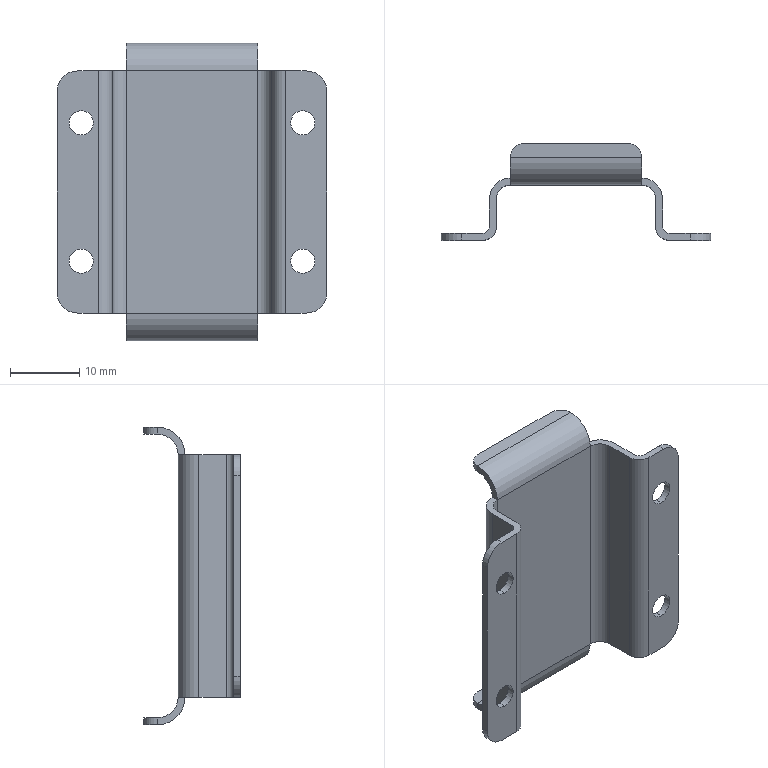Part | SolidWorks | features BaseBody 1 | 1 solid | 54 faces | box 39 x 14 x 43 mm | volume 2040 mm3 | cylinder 28 | plane 26 | commonest cylinder face diameters 3.5 x8 4 x8 6 x8 2 x2 8 x2
STEP:
#1=CARTESIAN_POINT('',(-16.,-9.,-11.75));
#2=VERTEX_POINT('',#1);
#3=CARTESIAN_POINT('',(-16.,-9.,-8.25));
#4=VERTEX_POINT('',#3);
#5=CARTESIAN_POINT('',(-16.,-9.,-10.));
#6=DIRECTION('',(0.,1.,0.));
#7=DIRECTION('',(-1.,0.,0.));
#8=AXIS2_PLACEMENT_3D('',#5,#6,#7);
#9=CIRCLE('',#8,1.75);
#10=EDGE_CURVE('',#2,#4,#9,.T.);
#11=ORIENTED_EDGE('',*,*,#10,.F.);
#12=CARTESIAN_POINT('',(-16.,-8.,-11.75));
#13=VERTEX_POINT('',#12);
#14=CARTESIAN_POINT('',(-16.,-8.,-11.75));
#15=DIRECTION('',(0.,1.,0.));
#16=VECTOR('',#15,1000.);
#17=LINE('',#14,#16);
#18=EDGE_CURVE('',#2,#13,#17,.T.);
#19=ORIENTED_EDGE('',*,*,#18,.T.);
#20=CARTESIAN_POINT('',(-16.,-8.,-8.25));
#21=VERTEX_POINT('',#20);
#22=CARTESIAN_POINT('',(-16.,-8.,-10.));
#23=DIRECTION('',(0.,1.,0.));
#24=DIRECTION('',(0.,0.,1.));
#25=AXIS2_PLACEMENT_3D('',#22,#23,#24);
#26=CIRCLE('',#25,1.75);
#27=EDGE_CURVE('',#13,#21,#26,.T.);
#28=ORIENTED_EDGE('',*,*,#27,.T.);
#29=CARTESIAN_POINT('',(-16.,-8.,-8.25));
#30=DIRECTION('',(0.,1.,0.));
#31=VECTOR('',#30,1000.);
#32=LINE('',#29,#31);
#33=EDGE_CURVE('',#4,#21,#32,.T.);
#34=ORIENTED_EDGE('',*,*,#33,.F.);
#35=EDGE_LOOP('',(#11,#19,#28,#34));
#36=FACE_OUTER_BOUND('',#35,.T.);
#37=CARTESIAN_POINT('',(-16.,-8.,-10.));
#38=DIRECTION('',(0.,1.,0.));
#39=DIRECTION('',(0.,0.,1.));
#40=AXIS2_PLACEMENT_3D('',#37,#38,#39);
#41=CYLINDRICAL_SURFACE('',#40,1.75);
#42=ADVANCED_FACE('',(#36),#41,.F.);
#43=CARTESIAN_POINT('',(-16.,-9.,8.25));
#44=VERTEX_POINT('',#43);
#45=CARTESIAN_POINT('',(-16.,-9.,11.75));
#46=VERTEX_POINT('',#45);
#47=CARTESIAN_POINT('',(-16.,-9.,10.));
#48=DIRECTION('',(0.,1.,0.));
#49=DIRECTION('',(-1.,0.,0.));
#50=AXIS2_PLACEMENT_3D('',#47,#48,#49);
#51=CIRCLE('',#50,1.75);
#52=EDGE_CURVE('',#44,#46,#51,.T.);
#53=ORIENTED_EDGE('',*,*,#52,.F.);
#54=CARTESIAN_POINT('',(-16.,-8.,8.25));
#55=VERTEX_POINT('',#54);
#56=CARTESIAN_POINT('',(-16.,-8.,8.25));
#57=DIRECTION('',(0.,1.,0.));
#58=VECTOR('',#57,1000.);
#59=LINE('',#56,#58);
#60=EDGE_CURVE('',#44,#55,#59,.T.);
#61=ORIENTED_EDGE('',*,*,#60,.T.);
#62=CARTESIAN_POINT('',(-16.,-8.,11.75));
#63=VERTEX_POINT('',#62);
#64=CARTESIAN_POINT('',(-16.,-8.,10.));
#65=DIRECTION('',(0.,1.,0.));
#66=DIRECTION('',(0.,0.,1.));
#67=AXIS2_PLACEMENT_3D('',#64,#65,#66);
#68=CIRCLE('',#67,1.75);
#69=EDGE_CURVE('',#55,#63,#68,.T.);
#70=ORIENTED_EDGE('',*,*,#69,.T.);
#71=CARTESIAN_POINT('',(-16.,-8.,11.75));
#72=DIRECTION('',(0.,1.,0.));
#73=VECTOR('',#72,1000.);
#74=LINE('',#71,#73);
#75=EDGE_CURVE('',#46,#63,#74,.T.);
#76=ORIENTED_EDGE('',*,*,#75,.F.);
#77=EDGE_LOOP('',(#53,#61,#70,#76));
#78=FACE_OUTER_BOUND('',#77,.T.);
#79=CARTESIAN_POINT('',(-16.,-8.,10.));
#80=DIRECTION('',(0.,1.,0.));
#81=DIRECTION('',(0.,0.,1.));
#82=AXIS2_PLACEMENT_3D('',#79,#80,#81);
#83=CYLINDRICAL_SURFACE('',#82,1.75);
#84=ADVANCED_FACE('',(#78),#83,.F.);
#85=CARTESIAN_POINT('',(16.,-9.,8.25));
#86=VERTEX_POINT('',#85);
#87=CARTESIAN_POINT('',(16.,-9.,11.75));
#88=VERTEX_POINT('',#87);
#89=CARTESIAN_POINT('',(16.,-9.,10.));
#90=DIRECTION('',(0.,1.,0.));
#91=DIRECTION('',(0.,0.,1.));
#92=AXIS2_PLACEMENT_3D('',#89,#90,#91);
#93=CIRCLE('',#92,1.75);
#94=EDGE_CURVE('',#86,#88,#93,.T.);
#95=ORIENTED_EDGE('',*,*,#94,.F.);
#96=CARTESIAN_POINT('',(16.,-8.,8.25));
#97=VERTEX_POINT('',#96);
#98=CARTESIAN_POINT('',(16.,-8.,8.25));
#99=DIRECTION('',(0.,1.,0.));
#100=VECTOR('',#99,1000.);
#101=LINE('',#98,#100);
#102=EDGE_CURVE('',#86,#97,#101,.T.);
#103=ORIENTED_EDGE('',*,*,#102,.T.);
#104=CARTESIAN_POINT('',(16.,-8.,11.75));
#105=VERTEX_POINT('',#104);
#106=CARTESIAN_POINT('',(16.,-8.,10.));
#107=DIRECTION('',(0.,1.,0.));
#108=DIRECTION('',(0.,0.,1.));
#109=AXIS2_PLACEMENT_3D('',#106,#107,#108);
#110=CIRCLE('',#109,1.75);
#111=EDGE_CURVE('',#97,#105,#110,.T.);
#112=ORIENTED_EDGE('',*,*,#111,.T.);
#113=CARTESIAN_POINT('',(16.,-8.,11.75));
#114=DIRECTION('',(0.,1.,0.));
#115=VECTOR('',#114,1000.);
#116=LINE('',#113,#115);
#117=EDGE_CURVE('',#88,#105,#116,.T.);
#118=ORIENTED_EDGE('',*,*,#117,.F.);
#119=EDGE_LOOP('',(#95,#103,#112,#118));
#120=FACE_OUTER_BOUND('',#119,.T.);
#121=CARTESIAN_POINT('',(16.,-8.,10.));
#122=DIRECTION('',(0.,1.,0.));
#123=DIRECTION('',(0.,0.,1.));
#124=AXIS2_PLACEMENT_3D('',#121,#122,#123);
#125=CYLINDRICAL_SURFACE('',#124,1.75);
#126=ADVANCED_FACE('',(#120),#125,.F.);
#127=CARTESIAN_POINT('',(16.,-9.,-11.75));
#128=VERTEX_POINT('',#127);
#129=CARTESIAN_POINT('',(16.,-9.,-8.25));
#130=VERTEX_POINT('',#129);
#131=CARTESIAN_POINT('',(16.,-9.,-10.));
#132=DIRECTION('',(0.,1.,0.));
#133=DIRECTION('',(0.,0.,1.));
#134=AXIS2_PLACEMENT_3D('',#131,#132,#133);
#135=CIRCLE('',#134,1.75);
#136=EDGE_CURVE('',#128,#130,#135,.T.);
#137=ORIENTED_EDGE('',*,*,#136,.F.);
#138=CARTESIAN_POINT('',(16.,-8.,-11.75));
#139=VERTEX_POINT('',#138);
#140=CARTESIAN_POINT('',(16.,-8.,-11.75));
#141=DIRECTION('',(0.,1.,0.));
#142=VECTOR('',#141,1000.);
#143=LINE('',#140,#142);
#144=EDGE_CURVE('',#128,#139,#143,.T.);
#145=ORIENTED_EDGE('',*,*,#144,.T.);
#146=CARTESIAN_POINT('',(16.,-8.,-8.25));
#147=VERTEX_POINT('',#146);
#148=CARTESIAN_POINT('',(16.,-8.,-10.));
#149=DIRECTION('',(0.,1.,0.));
#150=DIRECTION('',(0.,0.,1.));
#151=AXIS2_PLACEMENT_3D('',#148,#149,#150);
#152=CIRCLE('',#151,1.75);
#153=EDGE_CURVE('',#139,#147,#152,.T.);
#154=ORIENTED_EDGE('',*,*,#153,.T.);
#155=CARTESIAN_POINT('',(16.,-8.,-8.25));
#156=DIRECTION('',(0.,1.,0.));
#157=VECTOR('',#156,1000.);
#158=LINE('',#155,#157);
#159=EDGE_CURVE('',#130,#147,#158,.T.);
#160=ORIENTED_EDGE('',*,*,#159,.F.);
#161=EDGE_LOOP('',(#137,#145,#154,#160));
#162=FACE_OUTER_BOUND('',#161,.T.);
#163=CARTESIAN_POINT('',(16.,-8.,-10.));
#164=DIRECTION('',(0.,1.,0.));
#165=DIRECTION('',(0.,0.,1.));
#166=AXIS2_PLACEMENT_3D('',#163,#164,#165);
#167=CYLINDRICAL_SURFACE('',#166,1.75);
#168=ADVANCED_FACE('',(#162),#167,.F.);
#169=CARTESIAN_POINT('',(9.5,3.,21.5));
#170=VERTEX_POINT('',#169);
#171=CARTESIAN_POINT('',(7.5,5.,21.5));
#172=VERTEX_POINT('',#171);
#173=CARTESIAN_POINT('',(7.5,3.,21.5));
#174=DIRECTION('',(0.,0.,1.));
#175=DIRECTION('',(-1.,0.,0.));
#176=AXIS2_PLACEMENT_3D('',#173,#174,#175);
#177=CIRCLE('',#176,2.);
#178=EDGE_CURVE('',#170,#172,#177,.T.);
#179=ORIENTED_EDGE('',*,*,#178,.F.);
#180=CARTESIAN_POINT('',(9.5,3.,20.5));
#181=VERTEX_POINT('',#180);
#182=CARTESIAN_POINT('',(9.5,3.,20.5));
#183=DIRECTION('',(0.,0.,1.));
#184=VECTOR('',#183,1000.);
#185=LINE('',#182,#184);
#186=EDGE_CURVE('',#181,#170,#185,.T.);
#187=ORIENTED_EDGE('',*,*,#186,.F.);
#188=CARTESIAN_POINT('',(7.5,5.,20.5));
#189=VERTEX_POINT('',#188);
#190=CARTESIAN_POINT('',(7.5,3.,20.5));
#191=DIRECTION('',(0.,0.,-1.));
#192=DIRECTION('',(-1.,0.,0.));
#193=AXIS2_PLACEMENT_3D('',#190,#191,#192);
#194=CIRCLE('',#193,2.);
#195=EDGE_CURVE('',#189,#181,#194,.T.);
#196=ORIENTED_EDGE('',*,*,#195,.F.);
#197=CARTESIAN_POINT('',(7.5,5.,21.5));
#198=DIRECTION('',(0.,0.,-1.));
#199=VECTOR('',#198,1000.);
#200=LINE('',#197,#199);
#201=EDGE_CURVE('',#172,#189,#200,.T.);
#202=ORIENTED_EDGE('',*,*,#201,.F.);
#203=EDGE_LOOP('',(#179,#187,#196,#202));
#204=FACE_OUTER_BOUND('',#203,.T.);
#205=CARTESIAN_POINT('',(7.5,3.,21.5));
#206=DIRECTION('',(0.,0.,-1.));
#207=DIRECTION('',(-1.,0.,0.));
#208=AXIS2_PLACEMENT_3D('',#205,#206,#207);
#209=CYLINDRICAL_SURFACE('',#208,2.);
#210=ADVANCED_FACE('',(#204),#209,.T.);
#211=CARTESIAN_POINT('',(-7.5,5.,21.5));
#212=VERTEX_POINT('',#211);
#213=CARTESIAN_POINT('',(-9.5,3.,21.5));
#214=VERTEX_POINT('',#213);
#215=CARTESIAN_POINT('',(-7.5,3.,21.5));
#216=DIRECTION('',(0.,0.,1.));
#217=DIRECTION('',(-1.,0.,0.));
#218=AXIS2_PLACEMENT_3D('',#215,#216,#217);
#219=CIRCLE('',#218,2.);
#220=EDGE_CURVE('',#212,#214,#219,.T.);
#221=ORIENTED_EDGE('',*,*,#220,.F.);
#222=CARTESIAN_POINT('',(-7.5,5.,20.5));
#223=VERTEX_POINT('',#222);
#224=CARTESIAN_POINT('',(-7.5,5.,21.5));
#225=DIRECTION('',(0.,0.,1.));
#226=VECTOR('',#225,1000.);
#227=LINE('',#224,#226);
#228=EDGE_CURVE('',#223,#212,#227,.T.);
#229=ORIENTED_EDGE('',*,*,#228,.F.);
#230=CARTESIAN_POINT('',(-9.5,3.,20.5));
#231=VERTEX_POINT('',#230);
#232=CARTESIAN_POINT('',(-7.5,3.,20.5));
#233=DIRECTION('',(0.,0.,-1.));
#234=DIRECTION('',(-1.,0.,0.));
#235=AXIS2_PLACEMENT_3D('',#232,#233,#234);
#236=CIRCLE('',#235,2.);
#237=EDGE_CURVE('',#231,#223,#236,.T.);
#238=ORIENTED_EDGE('',*,*,#237,.F.);
#239=CARTESIAN_POINT('',(-9.5,3.,21.5));
#240=DIRECTION('',(0.,0.,1.));
#241=VECTOR('',#240,1000.);
#242=LINE('',#239,#241);
#243=EDGE_CURVE('',#231,#214,#242,.T.);
#244=ORIENTED_EDGE('',*,*,#243,.T.);
#245=EDGE_LOOP('',(#221,#229,#238,#244));
#246=FACE_OUTER_BOUND('',#245,.T.);
#247=CARTESIAN_POINT('',(-7.5,3.,21.5));
#248=DIRECTION('',(0.,0.,-1.));
#249=DIRECTION('',(-1.,0.,0.));
#250=AXIS2_PLACEMENT_3D('',#247,#248,#249);
#251=CYLINDRICAL_SURFACE('',#250,2.);
#252=ADVANCED_FACE('',(#246),#251,.T.);
#253=CARTESIAN_POINT('',(7.5,5.,-21.5));
#254=VERTEX_POINT('',#253);
#255=CARTESIAN_POINT('',(9.5,3.,-21.5));
#256=VERTEX_POINT('',#255);
#257=CARTESIAN_POINT('',(7.5,3.,-21.5));
#258=DIRECTION('',(0.,0.,-1.));
#259=DIRECTION('',(0.,-1.,0.));
#260=AXIS2_PLACEMENT_3D('',#257,#258,#259);
#261=CIRCLE('',#260,2.);
#262=EDGE_CURVE('',#254,#256,#261,.T.);
#263=ORIENTED_EDGE('',*,*,#262,.F.);
#264=CARTESIAN_POINT('',(7.5,5.,-20.5));
#265=VERTEX_POINT('',#264);
#266=CARTESIAN_POINT('',(7.5,5.,-21.5));
#267=DIRECTION('',(0.,0.,-1.));
#268=VECTOR('',#267,1000.);
#269=LINE('',#266,#268);
#270=EDGE_CURVE('',#265,#254,#269,.T.);
#271=ORIENTED_EDGE('',*,*,#270,.F.);
#272=CARTESIAN_POINT('',(9.5,3.,-20.5));
#273=VERTEX_POINT('',#272);
#274=CARTESIAN_POINT('',(7.5,3.,-20.5));
#275=DIRECTION('',(0.,0.,1.));
#276=DIRECTION('',(0.,-1.,0.));
#277=AXIS2_PLACEMENT_3D('',#274,#275,#276);
#278=CIRCLE('',#277,2.);
#279=EDGE_CURVE('',#273,#265,#278,.T.);
#280=ORIENTED_EDGE('',*,*,#279,.F.);
#281=CARTESIAN_POINT('',(9.5,3.,-21.5));
#282=DIRECTION('',(0.,0.,-1.));
#283=VECTOR('',#282,1000.);
#284=LINE('',#281,#283);
#285=EDGE_CURVE('',#273,#256,#284,.T.);
#286=ORIENTED_EDGE('',*,*,#285,.T.);
#287=EDGE_LOOP('',(#263,#271,#280,#286));
#288=FACE_OUTER_BOUND('',#287,.T.);
#289=CARTESIAN_POINT('',(7.5,3.,-21.5));
#290=DIRECTION('',(0.,0.,1.));
#291=DIRECTION('',(0.,-1.,0.));
#292=AXIS2_PLACEMENT_3D('',#289,#290,#291);
#293=CYLINDRICAL_SURFACE('',#292,2.);
#294=ADVANCED_FACE('',(#288),#293,.T.);
#295=CARTESIAN_POINT('',(-9.5,3.,-21.5));
#296=VERTEX_POINT('',#295);
#297=CARTESIAN_POINT('',(-7.5,5.,-21.5));
#298=VERTEX_POINT('',#297);
#299=CARTESIAN_POINT('',(-7.5,3.,-21.5));
#300=DIRECTION('',(0.,0.,-1.));
#301=DIRECTION('',(0.,-1.,0.));
#302=AXIS2_PLACEMENT_3D('',#299,#300,#301);
#303=CIRCLE('',#302,2.);
#304=EDGE_CURVE('',#296,#298,#303,.T.);
#305=ORIENTED_EDGE('',*,*,#304,.F.);
#306=CARTESIAN_POINT('',(-9.5,3.,-20.5));
#307=VERTEX_POINT('',#306);
#308=CARTESIAN_POINT('',(-9.5,3.,-20.5));
#309=DIRECTION('',(0.,0.,-1.));
#310=VECTOR('',#309,1000.);
#311=LINE('',#308,#310);
#312=EDGE_CURVE('',#307,#296,#311,.T.);
#313=ORIENTED_EDGE('',*,*,#312,.F.);
#314=CARTESIAN_POINT('',(-7.5,5.,-20.5));
#315=VERTEX_POINT('',#314);
#316=CARTESIAN_POINT('',(-7.5,3.,-20.5));
#317=DIRECTION('',(0.,0.,1.));
#318=DIRECTION('',(0.,-1.,0.));
#319=AXIS2_PLACEMENT_3D('',#316,#317,#318);
#320=CIRCLE('',#319,2.);
#321=EDGE_CURVE('',#315,#307,#320,.T.);
#322=ORIENTED_EDGE('',*,*,#321,.F.);
#323=CARTESIAN_POINT('',(-7.5,5.,-21.5));
#324=DIRECTION('',(0.,0.,1.));
#325=VECTOR('',#324,1000.);
#326=LINE('',#323,#325);
#327=EDGE_CURVE('',#298,#315,#326,.T.);
#328=ORIENTED_EDGE('',*,*,#327,.F.);
#329=EDGE_LOOP('',(#305,#313,#322,#328));
#330=FACE_OUTER_BOUND('',#329,.T.);
#331=CARTESIAN_POINT('',(-7.5,3.,-21.5));
#332=DIRECTION('',(0.,0.,1.));
#333=DIRECTION('',(0.,-1.,0.));
#334=AXIS2_PLACEMENT_3D('',#331,#332,#333);
#335=CYLINDRICAL_SURFACE('',#334,2.);
#336=ADVANCED_FACE('',(#330),#335,.T.);
#337=CARTESIAN_POINT('',(-9.5,5.,20.5));
#338=DIRECTION('',(-1.,0.,0.));
#339=VECTOR('',#338,1000.);
#340=LINE('',#337,#339);
#341=EDGE_CURVE('',#189,#223,#340,.T.);
#342=ORIENTED_EDGE('',*,*,#341,.T.);
#343=ORIENTED_EDGE('',*,*,#228,.T.);
#344=CARTESIAN_POINT('',(0.,5.,21.5));
#345=DIRECTION('',(-1.,0.,0.));
#346=VECTOR('',#345,1000.);
#347=LINE('',#344,#346);
#348=EDGE_CURVE('',#172,#212,#347,.T.);
#349=ORIENTED_EDGE('',*,*,#348,.F.);
#350=ORIENTED_EDGE('',*,*,#201,.T.);
#351=EDGE_LOOP('',(#342,#343,#349,#350));
#352=FACE_OUTER_BOUND('',#351,.T.);
#353=CARTESIAN_POINT('',(-9.5,5.,21.5));
#354=DIRECTION('',(0.,-1.,0.));
#355=DIRECTION('',(0.,0.,-1.));
#356=AXIS2_PLACEMENT_3D('',#353,#354,#355);
#357=PLANE('',#356);
#358=ADVANCED_FACE('',(#352),#357,.F.);
#359=CARTESIAN_POINT('',(-9.5,3.,20.5));
#360=DIRECTION('',(1.,0.,0.));
#361=VECTOR('',#360,1000.);
#362=LINE('',#359,#361);
#363=EDGE_CURVE('',#231,#181,#362,.T.);
#364=ORIENTED_EDGE('',*,*,#363,.F.);
#365=ORIENTED_EDGE('',*,*,#237,.T.);
#366=ORIENTED_EDGE('',*,*,#341,.F.);
#367=ORIENTED_EDGE('',*,*,#195,.T.);
#368=EDGE_LOOP('',(#364,#365,#366,#367));
#369=FACE_OUTER_BOUND('',#368,.T.);
#370=CARTESIAN_POINT('',(0.,0.,20.5));
#371=DIRECTION('',(0.,0.,-1.));
#372=DIRECTION('',(0.,-1.,0.));
#373=AXIS2_PLACEMENT_3D('',#370,#371,#372);
#374=PLANE('',#373);
#375=ADVANCED_FACE('',(#369),#374,.T.);
#376=ORIENTED_EDGE('',*,*,#348,.T.);
#377=ORIENTED_EDGE('',*,*,#220,.T.);
#378=CARTESIAN_POINT('',(-9.5,3.,21.5));
#379=DIRECTION('',(-1.,0.,0.));
#380=VECTOR('',#379,1000.);
#381=LINE('',#378,#380);
#382=EDGE_CURVE('',#170,#214,#381,.T.);
#383=ORIENTED_EDGE('',*,*,#382,.F.);
#384=ORIENTED_EDGE('',*,*,#178,.T.);
#385=EDGE_LOOP('',(#376,#377,#383,#384));
#386=FACE_OUTER_BOUND('',#385,.T.);
#387=CARTESIAN_POINT('',(0.,0.,21.5));
#388=DIRECTION('',(0.,0.,-1.));
#389=DIRECTION('',(0.,-1.,0.));
#390=AXIS2_PLACEMENT_3D('',#387,#388,#389);
#391=PLANE('',#390);
#392=ADVANCED_FACE('',(#386),#391,.F.);
#393=CARTESIAN_POINT('',(-9.5,0.,17.5));
#394=VERTEX_POINT('',#393);
#395=CARTESIAN_POINT('',(9.5,0.,17.5));
#396=VERTEX_POINT('',#395);
#397=CARTESIAN_POINT('',(-11.5,0.,17.5));
#398=DIRECTION('',(1.,0.,0.));
#399=VECTOR('',#398,1000.);
#400=LINE('',#397,#399);
#401=EDGE_CURVE('',#394,#396,#400,.T.);
#402=ORIENTED_EDGE('',*,*,#401,.F.);
#403=CARTESIAN_POINT('',(-9.5,3.,17.5));
#404=DIRECTION('',(-1.,0.,0.));
#405=DIRECTION('',(0.,0.,-1.));
#406=AXIS2_PLACEMENT_3D('',#403,#404,#405);
#407=CIRCLE('',#406,3.);
#408=EDGE_CURVE('',#394,#231,#407,.T.);
#409=ORIENTED_EDGE('',*,*,#408,.T.);
#410=ORIENTED_EDGE('',*,*,#363,.T.);
#411=CARTESIAN_POINT('',(9.5,3.,17.5));
#412=DIRECTION('',(1.,0.,0.));
#413=DIRECTION('',(0.,0.,-1.));
#414=AXIS2_PLACEMENT_3D('',#411,#412,#413);
#415=CIRCLE('',#414,3.);
#416=EDGE_CURVE('',#181,#396,#415,.T.);
#417=ORIENTED_EDGE('',*,*,#416,.T.);
#418=EDGE_LOOP('',(#402,#409,#410,#417));
#419=FACE_OUTER_BOUND('',#418,.T.);
#420=CARTESIAN_POINT('',(9.5,3.,17.5));
#421=DIRECTION('',(1.,0.,0.));
#422=DIRECTION('',(0.,0.,1.));
#423=AXIS2_PLACEMENT_3D('',#420,#421,#422);
#424=CYLINDRICAL_SURFACE('',#423,3.);
#425=ADVANCED_FACE('',(#419),#424,.F.);
#426=CARTESIAN_POINT('',(-9.5,-1.,17.5));
#427=VERTEX_POINT('',#426);
#428=CARTESIAN_POINT('',(9.5,-1.,17.5));
#429=VERTEX_POINT('',#428);
#430=CARTESIAN_POINT('',(-11.5,-1.,17.5));
#431=DIRECTION('',(1.,0.,0.));
#432=VECTOR('',#431,1000.);
#433=LINE('',#430,#432);
#434=EDGE_CURVE('',#427,#429,#433,.T.);
#435=ORIENTED_EDGE('',*,*,#434,.T.);
#436=CARTESIAN_POINT('',(9.5,3.,17.5));
#437=DIRECTION('',(1.,0.,0.));
#438=DIRECTION('',(0.,0.,-1.));
#439=AXIS2_PLACEMENT_3D('',#436,#437,#438);
#440=CIRCLE('',#439,4.);
#441=EDGE_CURVE('',#170,#429,#440,.T.);
#442=ORIENTED_EDGE('',*,*,#441,.F.);
#443=ORIENTED_EDGE('',*,*,#382,.T.);
#444=CARTESIAN_POINT('',(-9.5,3.,17.5));
#445=DIRECTION('',(-1.,0.,0.));
#446=DIRECTION('',(0.,0.,-1.));
#447=AXIS2_PLACEMENT_3D('',#444,#445,#446);
#448=CIRCLE('',#447,4.);
#449=EDGE_CURVE('',#427,#214,#448,.T.);
#450=ORIENTED_EDGE('',*,*,#449,.F.);
#451=EDGE_LOOP('',(#435,#442,#443,#450));
#452=FACE_OUTER_BOUND('',#451,.T.);
#453=CARTESIAN_POINT('',(9.5,3.,17.5));
#454=DIRECTION('',(1.,0.,0.));
#455=DIRECTION('',(0.,0.,1.));
#456=AXIS2_PLACEMENT_3D('',#453,#454,#455);
#457=CYLINDRICAL_SURFACE('',#456,4.);
#458=ADVANCED_FACE('',(#452),#457,.T.);
#459=ORIENTED_EDGE('',*,*,#416,.F.);
#460=ORIENTED_EDGE('',*,*,#186,.T.);
#461=ORIENTED_EDGE('',*,*,#441,.T.);
#462=CARTESIAN_POINT('',(9.5,-1.,17.5));
#463=DIRECTION('',(0.,1.,0.));
#464=VECTOR('',#463,1000.);
#465=LINE('',#462,#464);
#466=EDGE_CURVE('',#429,#396,#465,.T.);
#467=ORIENTED_EDGE('',*,*,#466,.T.);
#468=EDGE_LOOP('',(#459,#460,#461,#467));
#469=FACE_OUTER_BOUND('',#468,.T.);
#470=CARTESIAN_POINT('',(9.5,3.,17.5));
#471=DIRECTION('',(-1.,0.,0.));
#472=DIRECTION('',(0.,0.,1.));
#473=AXIS2_PLACEMENT_3D('',#470,#471,#472);
#474=PLANE('',#473);
#475=ADVANCED_FACE('',(#469),#474,.F.);
#476=ORIENTED_EDGE('',*,*,#243,.F.);
#477=ORIENTED_EDGE('',*,*,#408,.F.);
#478=CARTESIAN_POINT('',(-9.5,-1.,17.5));
#479=DIRECTION('',(0.,1.,0.));
#480=VECTOR('',#479,1000.);
#481=LINE('',#478,#480);
#482=EDGE_CURVE('',#427,#394,#481,.T.);
#483=ORIENTED_EDGE('',*,*,#482,.F.);
#484=ORIENTED_EDGE('',*,*,#449,.T.);
#485=EDGE_LOOP('',(#476,#477,#483,#484));
#486=FACE_OUTER_BOUND('',#485,.T.);
#487=CARTESIAN_POINT('',(-9.5,3.,17.5));
#488=DIRECTION('',(-1.,0.,0.));
#489=DIRECTION('',(0.,0.,1.));
#490=AXIS2_PLACEMENT_3D('',#487,#488,#489);
#491=PLANE('',#490);
#492=ADVANCED_FACE('',(#486),#491,.T.);
#493=CARTESIAN_POINT('',(0.,5.,-21.5));
#494=DIRECTION('',(1.,0.,0.));
#495=VECTOR('',#494,1000.);
#496=LINE('',#493,#495);
#497=EDGE_CURVE('',#298,#254,#496,.T.);
#498=ORIENTED_EDGE('',*,*,#497,.F.);
#499=ORIENTED_EDGE('',*,*,#327,.T.);
#500=CARTESIAN_POINT('',(9.5,5.,-20.5));
#501=DIRECTION('',(1.,0.,0.));
#502=VECTOR('',#501,1000.);
#503=LINE('',#500,#502);
#504=EDGE_CURVE('',#315,#265,#503,.T.);
#505=ORIENTED_EDGE('',*,*,#504,.T.);
#506=ORIENTED_EDGE('',*,*,#270,.T.);
#507=EDGE_LOOP('',(#498,#499,#505,#506));
#508=FACE_OUTER_BOUND('',#507,.T.);
#509=CARTESIAN_POINT('',(9.5,5.,-21.5));
#510=DIRECTION('',(0.,-1.,0.));
#511=DIRECTION('',(-1.,0.,0.));
#512=AXIS2_PLACEMENT_3D('',#509,#510,#511);
#513=PLANE('',#512);
#514=ADVANCED_FACE('',(#508),#513,.F.);
#515=ORIENTED_EDGE('',*,*,#504,.F.);
#516=ORIENTED_EDGE('',*,*,#321,.T.);
#517=CARTESIAN_POINT('',(9.5,3.,-20.5));
#518=DIRECTION('',(-1.,0.,0.));
#519=VECTOR('',#518,1000.);
#520=LINE('',#517,#519);
#521=EDGE_CURVE('',#273,#307,#520,.T.);
#522=ORIENTED_EDGE('',*,*,#521,.F.);
#523=ORIENTED_EDGE('',*,*,#279,.T.);
#524=EDGE_LOOP('',(#515,#516,#522,#523));
#525=FACE_OUTER_BOUND('',#524,.T.);
#526=CARTESIAN_POINT('',(0.,0.,-20.5));
#527=DIRECTION('',(0.,0.,1.));
#528=DIRECTION('',(0.,-1.,0.));
#529=AXIS2_PLACEMENT_3D('',#526,#527,#528);
#530=PLANE('',#529);
#531=ADVANCED_FACE('',(#525),#530,.T.);
#532=CARTESIAN_POINT('',(9.5,3.,-21.5));
#533=DIRECTION('',(1.,0.,0.));
#534=VECTOR('',#533,1000.);
#535=LINE('',#532,#534);
#536=EDGE_CURVE('',#296,#256,#535,.T.);
#537=ORIENTED_EDGE('',*,*,#536,.F.);
#538=ORIENTED_EDGE('',*,*,#304,.T.);
#539=ORIENTED_EDGE('',*,*,#497,.T.);
#540=ORIENTED_EDGE('',*,*,#262,.T.);
#541=EDGE_LOOP('',(#537,#538,#539,#540));
#542=FACE_OUTER_BOUND('',#541,.T.);
#543=CARTESIAN_POINT('',(0.,0.,-21.5));
#544=DIRECTION('',(0.,0.,1.));
#545=DIRECTION('',(0.,-1.,0.));
#546=AXIS2_PLACEMENT_3D('',#543,#544,#545);
#547=PLANE('',#546);
#548=ADVANCED_FACE('',(#542),#547,.F.);
#549=CARTESIAN_POINT('',(9.5,0.,-17.5));
#550=VERTEX_POINT('',#549);
#551=CARTESIAN_POINT('',(-9.5,0.,-17.5));
#552=VERTEX_POINT('',#551);
#553=CARTESIAN_POINT('',(-11.5,0.,-17.5));
#554=DIRECTION('',(-1.,0.,0.));
#555=VECTOR('',#554,1000.);
#556=LINE('',#553,#555);
#557=EDGE_CURVE('',#550,#552,#556,.T.);
#558=ORIENTED_EDGE('',*,*,#557,.F.);
#559=CARTESIAN_POINT('',(9.5,3.,-17.5));
#560=DIRECTION('',(1.,0.,0.));
#561=DIRECTION('',(0.,-1.,0.));
#562=AXIS2_PLACEMENT_3D('',#559,#560,#561);
#563=CIRCLE('',#562,3.);
#564=EDGE_CURVE('',#550,#273,#563,.T.);
#565=ORIENTED_EDGE('',*,*,#564,.T.);
#566=ORIENTED_EDGE('',*,*,#521,.T.);
#567=CARTESIAN_POINT('',(-9.5,3.,-17.5));
#568=DIRECTION('',(-1.,0.,0.));
#569=DIRECTION('',(0.,-1.,0.));
#570=AXIS2_PLACEMENT_3D('',#567,#568,#569);
#571=CIRCLE('',#570,3.);
#572=EDGE_CURVE('',#307,#552,#571,.T.);
#573=ORIENTED_EDGE('',*,*,#572,.T.);
#574=EDGE_LOOP('',(#558,#565,#566,#573));
#575=FACE_OUTER_BOUND('',#574,.T.);
#576=CARTESIAN_POINT('',(-9.5,3.,-17.5));
#577=DIRECTION('',(-1.,0.,0.));
#578=DIRECTION('',(0.,0.,-1.));
#579=AXIS2_PLACEMENT_3D('',#576,#577,#578);
#580=CYLINDRICAL_SURFACE('',#579,3.);
#581=ADVANCED_FACE('',(#575),#580,.F.);
#582=CARTESIAN_POINT('',(9.5,-1.,-17.5));
#583=VERTEX_POINT('',#582);
#584=CARTESIAN_POINT('',(-9.5,-1.,-17.5));
#585=VERTEX_POINT('',#584);
#586=CARTESIAN_POINT('',(-11.5,-1.,-17.5));
#587=DIRECTION('',(-1.,0.,0.));
#588=VECTOR('',#587,1000.);
#589=LINE('',#586,#588);
#590=EDGE_CURVE('',#583,#585,#589,.T.);
#591=ORIENTED_EDGE('',*,*,#590,.T.);
#592=CARTESIAN_POINT('',(-9.5,3.,-17.5));
#593=DIRECTION('',(-1.,0.,0.));
#594=DIRECTION('',(0.,-1.,0.));
#595=AXIS2_PLACEMENT_3D('',#592,#593,#594);
#596=CIRCLE('',#595,4.);
#597=EDGE_CURVE('',#296,#585,#596,.T.);
#598=ORIENTED_EDGE('',*,*,#597,.F.);
#599=ORIENTED_EDGE('',*,*,#536,.T.);
#600=CARTESIAN_POINT('',(9.5,3.,-17.5));
#601=DIRECTION('',(1.,0.,0.));
#602=DIRECTION('',(0.,-1.,0.));
#603=AXIS2_PLACEMENT_3D('',#600,#601,#602);
#604=CIRCLE('',#603,4.);
#605=EDGE_CURVE('',#583,#256,#604,.T.);
#606=ORIENTED_EDGE('',*,*,#605,.F.);
#607=EDGE_LOOP('',(#591,#598,#599,#606));
#608=FACE_OUTER_BOUND('',#607,.T.);
#609=CARTESIAN_POINT('',(-9.5,3.,-17.5));
#610=DIRECTION('',(-1.,0.,0.));
#611=DIRECTION('',(0.,0.,-1.));
#612=AXIS2_PLACEMENT_3D('',#609,#610,#611);
#613=CYLINDRICAL_SURFACE('',#612,4.);
#614=ADVANCED_FACE('',(#608),#613,.T.);
#615=ORIENTED_EDGE('',*,*,#572,.F.);
#616=ORIENTED_EDGE('',*,*,#312,.T.);
#617=ORIENTED_EDGE('',*,*,#597,.T.);
#618=CARTESIAN_POINT('',(-9.5,-1.,-17.5));
#619=DIRECTION('',(0.,1.,0.));
#620=VECTOR('',#619,1000.);
#621=LINE('',#618,#620);
#622=EDGE_CURVE('',#585,#552,#621,.T.);
#623=ORIENTED_EDGE('',*,*,#622,.T.);
#624=EDGE_LOOP('',(#615,#616,#617,#623));
#625=FACE_OUTER_BOUND('',#624,.T.);
#626=CARTESIAN_POINT('',(-9.5,3.,-17.5));
#627=DIRECTION('',(1.,0.,0.));
#628=DIRECTION('',(0.,1.,0.));
#629=AXIS2_PLACEMENT_3D('',#626,#627,#628);
#630=PLANE('',#629);
#631=ADVANCED_FACE('',(#625),#630,.F.);
#632=ORIENTED_EDGE('',*,*,#285,.F.);
#633=ORIENTED_EDGE('',*,*,#564,.F.);
#634=CARTESIAN_POINT('',(9.5,-1.,-17.5));
#635=DIRECTION('',(0.,1.,0.));
#636=VECTOR('',#635,1000.);
#637=LINE('',#634,#636);
#638=EDGE_CURVE('',#583,#550,#637,.T.);
#639=ORIENTED_EDGE('',*,*,#638,.F.);
#640=ORIENTED_EDGE('',*,*,#605,.T.);
#641=EDGE_LOOP('',(#632,#633,#639,#640));
#642=FACE_OUTER_BOUND('',#641,.T.);
#643=CARTESIAN_POINT('',(9.5,3.,-17.5));
#644=DIRECTION('',(1.,0.,0.));
#645=DIRECTION('',(0.,1.,0.));
#646=AXIS2_PLACEMENT_3D('',#643,#644,#645);
#647=PLANE('',#646);
#648=ADVANCED_FACE('',(#642),#647,.T.);
#649=CARTESIAN_POINT('',(16.5,-9.,-17.5));
#650=VERTEX_POINT('',#649);
#651=CARTESIAN_POINT('',(19.5,-9.,-14.5));
#652=VERTEX_POINT('',#651);
#653=CARTESIAN_POINT('',(16.5,-9.,-14.5));
#654=DIRECTION('',(0.,-1.,0.));
#655=DIRECTION('',(0.,0.,1.));
#656=AXIS2_PLACEMENT_3D('',#653,#654,#655);
#657=CIRCLE('',#656,3.);
#658=EDGE_CURVE('',#650,#652,#657,.T.);
#659=ORIENTED_EDGE('',*,*,#658,.F.);
#660=CARTESIAN_POINT('',(16.5,-8.,-17.5));
#661=VERTEX_POINT('',#660);
#662=CARTESIAN_POINT('',(16.5,-9.,-17.5));
#663=DIRECTION('',(0.,-1.,0.));
#664=VECTOR('',#663,1000.);
#665=LINE('',#662,#664);
#666=EDGE_CURVE('',#661,#650,#665,.T.);
#667=ORIENTED_EDGE('',*,*,#666,.F.);
#668=CARTESIAN_POINT('',(19.5,-8.,-14.5));
#669=VERTEX_POINT('',#668);
#670=CARTESIAN_POINT('',(16.5,-8.,-14.5));
#671=DIRECTION('',(0.,1.,0.));
#672=DIRECTION('',(0.,0.,1.));
#673=AXIS2_PLACEMENT_3D('',#670,#671,#672);
#674=CIRCLE('',#673,3.);
#675=EDGE_CURVE('',#669,#661,#674,.T.);
#676=ORIENTED_EDGE('',*,*,#675,.F.);
#677=CARTESIAN_POINT('',(19.5,-9.,-14.5));
#678=DIRECTION('',(0.,1.,0.));
#679=VECTOR('',#678,1000.);
#680=LINE('',#677,#679);
#681=EDGE_CURVE('',#652,#669,#680,.T.);
#682=ORIENTED_EDGE('',*,*,#681,.F.);
#683=EDGE_LOOP('',(#659,#667,#676,#682));
#684=FACE_OUTER_BOUND('',#683,.T.);
#685=CARTESIAN_POINT('',(16.5,-9.,-14.5));
#686=DIRECTION('',(0.,1.,0.));
#687=DIRECTION('',(-1.,0.,0.));
#688=AXIS2_PLACEMENT_3D('',#685,#686,#687);
#689=CYLINDRICAL_SURFACE('',#688,3.);
#690=ADVANCED_FACE('',(#684),#689,.T.);
#691=CARTESIAN_POINT('',(19.5,-9.,14.5));
#692=VERTEX_POINT('',#691);
#693=CARTESIAN_POINT('',(16.5,-9.,17.5));
#694=VERTEX_POINT('',#693);
#695=CARTESIAN_POINT('',(16.5,-9.,14.5));
#696=DIRECTION('',(0.,-1.,0.));
#697=DIRECTION('',(0.,0.,1.));
#698=AXIS2_PLACEMENT_3D('',#695,#696,#697);
#699=CIRCLE('',#698,3.);
#700=EDGE_CURVE('',#692,#694,#699,.T.);
#701=ORIENTED_EDGE('',*,*,#700,.F.);
#702=CARTESIAN_POINT('',(19.5,-8.,14.5));
#703=VERTEX_POINT('',#702);
#704=CARTESIAN_POINT('',(19.5,-9.,14.5));
#705=DIRECTION('',(0.,-1.,0.));
#706=VECTOR('',#705,1000.);
#707=LINE('',#704,#706);
#708=EDGE_CURVE('',#703,#692,#707,.T.);
#709=ORIENTED_EDGE('',*,*,#708,.F.);
#710=CARTESIAN_POINT('',(16.5,-8.,17.5));
#711=VERTEX_POINT('',#710);
#712=CARTESIAN_POINT('',(16.5,-8.,14.5));
#713=DIRECTION('',(0.,1.,0.));
#714=DIRECTION('',(0.,0.,1.));
#715=AXIS2_PLACEMENT_3D('',#712,#713,#714);
#716=CIRCLE('',#715,3.);
#717=EDGE_CURVE('',#711,#703,#716,.T.);
#718=ORIENTED_EDGE('',*,*,#717,.F.);
#719=CARTESIAN_POINT('',(16.5,-9.,17.5));
#720=DIRECTION('',(0.,1.,0.));
#721=VECTOR('',#720,1000.);
#722=LINE('',#719,#721);
#723=EDGE_CURVE('',#694,#711,#722,.T.);
#724=ORIENTED_EDGE('',*,*,#723,.F.);
#725=EDGE_LOOP('',(#701,#709,#718,#724));
#726=FACE_OUTER_BOUND('',#725,.T.);
#727=CARTESIAN_POINT('',(16.5,-9.,14.5));
#728=DIRECTION('',(0.,1.,0.));
#729=DIRECTION('',(-1.,0.,0.));
#730=AXIS2_PLACEMENT_3D('',#727,#728,#729);
#731=CYLINDRICAL_SURFACE('',#730,3.);
#732=ADVANCED_FACE('',(#726),#731,.T.);
#733=CARTESIAN_POINT('',(-16.5,-9.,17.5));
#734=VERTEX_POINT('',#733);
#735=CARTESIAN_POINT('',(-19.5,-9.,14.5));
#736=VERTEX_POINT('',#735);
#737=CARTESIAN_POINT('',(-16.5,-9.,14.5));
#738=DIRECTION('',(0.,-1.,0.));
#739=DIRECTION('',(-1.,0.,0.));
#740=AXIS2_PLACEMENT_3D('',#737,#738,#739);
#741=CIRCLE('',#740,3.);
#742=EDGE_CURVE('',#734,#736,#741,.T.);
#743=ORIENTED_EDGE('',*,*,#742,.F.);
#744=CARTESIAN_POINT('',(-16.5,-8.,17.5));
#745=VERTEX_POINT('',#744);
#746=CARTESIAN_POINT('',(-16.5,-9.,17.5));
#747=DIRECTION('',(0.,-1.,0.));
#748=VECTOR('',#747,1000.);
#749=LINE('',#746,#748);
#750=EDGE_CURVE('',#745,#734,#749,.T.);
#751=ORIENTED_EDGE('',*,*,#750,.F.);
#752=CARTESIAN_POINT('',(-19.5,-8.,14.5));
#753=VERTEX_POINT('',#752);
#754=CARTESIAN_POINT('',(-16.5,-8.,14.5));
#755=DIRECTION('',(0.,1.,0.));
#756=DIRECTION('',(-1.,0.,0.));
#757=AXIS2_PLACEMENT_3D('',#754,#755,#756);
#758=CIRCLE('',#757,3.);
#759=EDGE_CURVE('',#753,#745,#758,.T.);
#760=ORIENTED_EDGE('',*,*,#759,.F.);
#761=CARTESIAN_POINT('',(-19.5,-9.,14.5));
#762=DIRECTION('',(0.,1.,0.));
#763=VECTOR('',#762,1000.);
#764=LINE('',#761,#763);
#765=EDGE_CURVE('',#736,#753,#764,.T.);
#766=ORIENTED_EDGE('',*,*,#765,.F.);
#767=EDGE_LOOP('',(#743,#751,#760,#766));
#768=FACE_OUTER_BOUND('',#767,.T.);
#769=CARTESIAN_POINT('',(-16.5,-9.,14.5));
#770=DIRECTION('',(0.,1.,0.));
#771=DIRECTION('',(-1.,0.,0.));
#772=AXIS2_PLACEMENT_3D('',#769,#770,#771);
#773=CYLINDRICAL_SURFACE('',#772,3.);
#774=ADVANCED_FACE('',(#768),#773,.T.);
#775=CARTESIAN_POINT('',(-19.5,-9.,-14.5));
#776=VERTEX_POINT('',#775);
#777=CARTESIAN_POINT('',(-16.5,-9.,-17.5));
#778=VERTEX_POINT('',#777);
#779=CARTESIAN_POINT('',(-16.5,-9.,-14.5));
#780=DIRECTION('',(0.,-1.,0.));
#781=DIRECTION('',(-1.,0.,0.));
#782=AXIS2_PLACEMENT_3D('',#779,#780,#781);
#783=CIRCLE('',#782,3.);
#784=EDGE_CURVE('',#776,#778,#783,.T.);
#785=ORIENTED_EDGE('',*,*,#784,.F.);
#786=CARTESIAN_POINT('',(-19.5,-8.,-14.5));
#787=VERTEX_POINT('',#786);
#788=CARTESIAN_POINT('',(-19.5,-9.,-14.5));
#789=DIRECTION('',(0.,-1.,0.));
#790=VECTOR('',#789,1000.);
#791=LINE('',#788,#790);
#792=EDGE_CURVE('',#787,#776,#791,.T.);
#793=ORIENTED_EDGE('',*,*,#792,.F.);
#794=CARTESIAN_POINT('',(-16.5,-8.,-17.5));
#795=VERTEX_POINT('',#794);
#796=CARTESIAN_POINT('',(-16.5,-8.,-14.5));
#797=DIRECTION('',(0.,1.,0.));
#798=DIRECTION('',(-1.,0.,0.));
#799=AXIS2_PLACEMENT_3D('',#796,#797,#798);
#800=CIRCLE('',#799,3.);
#801=EDGE_CURVE('',#795,#787,#800,.T.);
#802=ORIENTED_EDGE('',*,*,#801,.F.);
#803=CARTESIAN_POINT('',(-16.5,-9.,-17.5));
#804=DIRECTION('',(0.,1.,0.));
#805=VECTOR('',#804,1000.);
#806=LINE('',#803,#805);
#807=EDGE_CURVE('',#778,#795,#806,.T.);
#808=ORIENTED_EDGE('',*,*,#807,.F.);
#809=EDGE_LOOP('',(#785,#793,#802,#808));
#810=FACE_OUTER_BOUND('',#809,.T.);
#811=CARTESIAN_POINT('',(-16.5,-9.,-14.5));
#812=DIRECTION('',(0.,1.,0.));
#813=DIRECTION('',(-1.,0.,0.));
#814=AXIS2_PLACEMENT_3D('',#811,#812,#813);
#815=CYLINDRICAL_SURFACE('',#814,3.);
#816=ADVANCED_FACE('',(#810),#815,.T.);
#817=CARTESIAN_POINT('',(-19.5,-8.,-17.5));
#818=DIRECTION('',(0.,0.,-1.));
#819=VECTOR('',#818,1000.);
#820=LINE('',#817,#819);
#821=EDGE_CURVE('',#753,#787,#820,.T.);
#822=ORIENTED_EDGE('',*,*,#821,.T.);
#823=ORIENTED_EDGE('',*,*,#792,.T.);
#824=CARTESIAN_POINT('',(-19.5,-9.,-17.5));
#825=DIRECTION('',(0.,0.,-1.));
#826=VECTOR('',#825,1000.);
#827=LINE('',#824,#826);
#828=EDGE_CURVE('',#736,#776,#827,.T.);
#829=ORIENTED_EDGE('',*,*,#828,.F.);
#830=ORIENTED_EDGE('',*,*,#765,.T.);
#831=EDGE_LOOP('',(#822,#823,#829,#830));
#832=FACE_OUTER_BOUND('',#831,.T.);
#833=CARTESIAN_POINT('',(-19.5,-9.,-17.5));
#834=DIRECTION('',(1.,0.,0.));
#835=DIRECTION('',(0.,-1.,0.));
#836=AXIS2_PLACEMENT_3D('',#833,#834,#835);
#837=PLANE('',#836);
#838=ADVANCED_FACE('',(#832),#837,.F.);
#839=CARTESIAN_POINT('',(-16.,-8.,10.));
#840=DIRECTION('',(0.,1.,0.));
#841=DIRECTION('',(0.,0.,1.));
#842=AXIS2_PLACEMENT_3D('',#839,#840,#841);
#843=CIRCLE('',#842,1.75);
#844=EDGE_CURVE('',#63,#55,#843,.T.);
#845=ORIENTED_EDGE('',*,*,#844,.F.);
#846=ORIENTED_EDGE('',*,*,#69,.F.);
#847=EDGE_LOOP('',(#845,#846));
#848=FACE_BOUND('',#847,.T.);
#849=CARTESIAN_POINT('',(-16.,-8.,-10.));
#850=DIRECTION('',(0.,1.,0.));
#851=DIRECTION('',(0.,0.,1.));
#852=AXIS2_PLACEMENT_3D('',#849,#850,#851);
#853=CIRCLE('',#852,1.75);
#854=EDGE_CURVE('',#21,#13,#853,.T.);
#855=ORIENTED_EDGE('',*,*,#854,.F.);
#856=ORIENTED_EDGE('',*,*,#27,.F.);
#857=EDGE_LOOP('',(#855,#856));
#858=FACE_BOUND('',#857,.T.);
#859=CARTESIAN_POINT('',(-13.5,-8.,-17.5));
#860=VERTEX_POINT('',#859);
#861=CARTESIAN_POINT('',(-12.5,-8.,-17.5));
#862=DIRECTION('',(1.,0.,0.));
#863=VECTOR('',#862,1000.);
#864=LINE('',#861,#863);
#865=EDGE_CURVE('',#795,#860,#864,.T.);
#866=ORIENTED_EDGE('',*,*,#865,.F.);
#867=ORIENTED_EDGE('',*,*,#801,.T.);
#868=ORIENTED_EDGE('',*,*,#821,.F.);
#869=ORIENTED_EDGE('',*,*,#759,.T.);
#870=CARTESIAN_POINT('',(-13.5,-8.,17.5));
#871=VERTEX_POINT('',#870);
#872=CARTESIAN_POINT('',(-19.5,-8.,17.5));
#873=DIRECTION('',(-1.,0.,0.));
#874=VECTOR('',#873,1000.);
#875=LINE('',#872,#874);
#876=EDGE_CURVE('',#871,#745,#875,.T.);
#877=ORIENTED_EDGE('',*,*,#876,.F.);
#878=CARTESIAN_POINT('',(-13.5,-8.,-17.5));
#879=DIRECTION('',(0.,0.,1.));
#880=VECTOR('',#879,1000.);
#881=LINE('',#878,#880);
#882=EDGE_CURVE('',#860,#871,#881,.T.);
#883=ORIENTED_EDGE('',*,*,#882,.F.);
#884=EDGE_LOOP('',(#866,#867,#868,#869,#877,#883));
#885=FACE_OUTER_BOUND('',#884,.T.);
#886=CARTESIAN_POINT('',(0.,-8.,0.));
#887=DIRECTION('',(0.,1.,0.));
#888=DIRECTION('',(1.,0.,0.));
#889=AXIS2_PLACEMENT_3D('',#886,#887,#888);
#890=PLANE('',#889);
#891=ADVANCED_FACE('',(#848,#858,#885),#890,.T.);
#892=CARTESIAN_POINT('',(-16.,-9.,10.));
#893=DIRECTION('',(0.,1.,0.));
#894=DIRECTION('',(-1.,0.,0.));
#895=AXIS2_PLACEMENT_3D('',#892,#893,#894);
#896=CIRCLE('',#895,1.75);
#897=EDGE_CURVE('',#46,#44,#896,.T.);
#898=ORIENTED_EDGE('',*,*,#897,.T.);
#899=ORIENTED_EDGE('',*,*,#52,.T.);
#900=EDGE_LOOP('',(#898,#899));
#901=FACE_BOUND('',#900,.T.);
#902=CARTESIAN_POINT('',(-16.,-9.,-10.));
#903=DIRECTION('',(0.,1.,0.));
#904=DIRECTION('',(-1.,0.,0.));
#905=AXIS2_PLACEMENT_3D('',#902,#903,#904);
#906=CIRCLE('',#905,1.75);
#907=EDGE_CURVE('',#4,#2,#906,.T.);
#908=ORIENTED_EDGE('',*,*,#907,.T.);
#909=ORIENTED_EDGE('',*,*,#10,.T.);
#910=EDGE_LOOP('',(#908,#909));
#911=FACE_BOUND('',#910,.T.);
#912=ORIENTED_EDGE('',*,*,#828,.T.);
#913=ORIENTED_EDGE('',*,*,#784,.T.);
#914=CARTESIAN_POINT('',(-13.5,-9.,-17.5));
#915=VERTEX_POINT('',#914);
#916=CARTESIAN_POINT('',(-12.5,-9.,-17.5));
#917=DIRECTION('',(1.,0.,0.));
#918=VECTOR('',#917,1000.);
#919=LINE('',#916,#918);
#920=EDGE_CURVE('',#778,#915,#919,.T.);
#921=ORIENTED_EDGE('',*,*,#920,.T.);
#922=CARTESIAN_POINT('',(-13.5,-9.,17.5));
#923=VERTEX_POINT('',#922);
#924=CARTESIAN_POINT('',(-13.5,-9.,0.));
#925=DIRECTION('',(0.,0.,-1.));
#926=VECTOR('',#925,1000.);
#927=LINE('',#924,#926);
#928=EDGE_CURVE('',#923,#915,#927,.T.);
#929=ORIENTED_EDGE('',*,*,#928,.F.);
#930=CARTESIAN_POINT('',(-19.5,-9.,17.5));
#931=DIRECTION('',(-1.,0.,0.));
#932=VECTOR('',#931,1000.);
#933=LINE('',#930,#932);
#934=EDGE_CURVE('',#923,#734,#933,.T.);
#935=ORIENTED_EDGE('',*,*,#934,.T.);
#936=ORIENTED_EDGE('',*,*,#742,.T.);
#937=EDGE_LOOP('',(#912,#913,#921,#929,#935,#936));
#938=FACE_OUTER_BOUND('',#937,.T.);
#939=CARTESIAN_POINT('',(0.,-9.,0.));
#940=DIRECTION('',(0.,1.,0.));
#941=DIRECTION('',(1.,0.,0.));
#942=AXIS2_PLACEMENT_3D('',#939,#940,#941);
#943=PLANE('',#942);
#944=ADVANCED_FACE('',(#901,#911,#938),#943,.F.);
#945=CARTESIAN_POINT('',(-12.5,-7.,17.5));
#946=VERTEX_POINT('',#945);
#947=CARTESIAN_POINT('',(-12.5,-7.,-17.5));
#948=VERTEX_POINT('',#947);
#949=CARTESIAN_POINT('',(-12.5,-7.,17.5));
#950=DIRECTION('',(0.,0.,-1.));
#951=VECTOR('',#950,1000.);
#952=LINE('',#949,#951);
#953=EDGE_CURVE('',#946,#948,#952,.T.);
#954=ORIENTED_EDGE('',*,*,#953,.T.);
#955=CARTESIAN_POINT('',(-13.5,-7.,-17.5));
#956=DIRECTION('',(0.,0.,-1.));
#957=DIRECTION('',(1.,0.,0.));
#958=AXIS2_PLACEMENT_3D('',#955,#956,#957);
#959=CIRCLE('',#958,1.);
#960=EDGE_CURVE('',#948,#860,#959,.T.);
#961=ORIENTED_EDGE('',*,*,#960,.T.);
#962=ORIENTED_EDGE('',*,*,#882,.T.);
#963=CARTESIAN_POINT('',(-13.5,-7.,17.5));
#964=DIRECTION('',(0.,0.,1.));
#965=DIRECTION('',(1.,0.,0.));
#966=AXIS2_PLACEMENT_3D('',#963,#964,#965);
#967=CIRCLE('',#966,1.);
#968=EDGE_CURVE('',#871,#946,#967,.T.);
#969=ORIENTED_EDGE('',*,*,#968,.T.);
#970=EDGE_LOOP('',(#954,#961,#962,#969));
#971=FACE_OUTER_BOUND('',#970,.T.);
#972=CARTESIAN_POINT('',(-13.5,-7.,17.5));
#973=DIRECTION('',(0.,0.,1.));
#974=DIRECTION('',(0.,-1.,0.));
#975=AXIS2_PLACEMENT_3D('',#972,#973,#974);
#976=CYLINDRICAL_SURFACE('',#975,1.);
#977=ADVANCED_FACE('',(#971),#976,.F.);
#978=CARTESIAN_POINT('',(-11.5,-7.,17.5));
#979=VERTEX_POINT('',#978);
#980=CARTESIAN_POINT('',(-11.5,-7.,-17.5));
#981=VERTEX_POINT('',#980);
#982=CARTESIAN_POINT('',(-11.5,-7.,17.5));
#983=DIRECTION('',(0.,0.,-1.));
#984=VECTOR('',#983,1000.);
#985=LINE('',#982,#984);
#986=EDGE_CURVE('',#979,#981,#985,.T.);
#987=ORIENTED_EDGE('',*,*,#986,.F.);
#988=CARTESIAN_POINT('',(-13.5,-7.,17.5));
#989=DIRECTION('',(0.,0.,1.));
#990=DIRECTION('',(1.,0.,0.));
#991=AXIS2_PLACEMENT_3D('',#988,#989,#990);
#992=CIRCLE('',#991,2.);
#993=EDGE_CURVE('',#923,#979,#992,.T.);
#994=ORIENTED_EDGE('',*,*,#993,.F.);
#995=ORIENTED_EDGE('',*,*,#928,.T.);
#996=CARTESIAN_POINT('',(-13.5,-7.,-17.5));
#997=DIRECTION('',(0.,0.,-1.));
#998=DIRECTION('',(1.,0.,0.));
#999=AXIS2_PLACEMENT_3D('',#996,#997,#998);
#1000=CIRCLE('',#999,2.);
#1001=EDGE_CURVE('',#981,#915,#1000,.T.);
#1002=ORIENTED_EDGE('',*,*,#1001,.F.);
#1003=EDGE_LOOP('',(#987,#994,#995,#1002));
#1004=FACE_OUTER_BOUND('',#1003,.T.);
#1005=CARTESIAN_POINT('',(-13.5,-7.,17.5));
#1006=DIRECTION('',(0.,0.,1.));
#1007=DIRECTION('',(0.,-1.,0.));
#1008=AXIS2_PLACEMENT_3D('',#1005,#1006,#1007);
#1009=CYLINDRICAL_SURFACE('',#1008,2.);
#1010=ADVANCED_FACE('',(#1004),#1009,.T.);
#1011=CARTESIAN_POINT('',(19.5,-8.,17.5));
#1012=DIRECTION('',(0.,0.,1.));
#1013=VECTOR('',#1012,1000.);
#1014=LINE('',#1011,#1013);
#1015=EDGE_CURVE('',#669,#703,#1014,.T.);
#1016=ORIENTED_EDGE('',*,*,#1015,.T.);
#1017=ORIENTED_EDGE('',*,*,#708,.T.);
#1018=CARTESIAN_POINT('',(19.5,-9.,17.5));
#1019=DIRECTION('',(0.,0.,1.));
#1020=VECTOR('',#1019,1000.);
#1021=LINE('',#1018,#1020);
#1022=EDGE_CURVE('',#652,#692,#1021,.T.);
#1023=ORIENTED_EDGE('',*,*,#1022,.F.);
#1024=ORIENTED_EDGE('',*,*,#681,.T.);
#1025=EDGE_LOOP('',(#1016,#1017,#1023,#1024));
#1026=FACE_OUTER_BOUND('',#1025,.T.);
#1027=CARTESIAN_POINT('',(19.5,-9.,17.5));
#1028=DIRECTION('',(-1.,0.,0.));
#1029=DIRECTION('',(0.,1.,0.));
#1030=AXIS2_PLACEMENT_3D('',#1027,#1028,#1029);
#1031=PLANE('',#1030);
#1032=ADVANCED_FACE('',(#1026),#1031,.F.);
#1033=CARTESIAN_POINT('',(16.,-8.,-10.));
#1034=DIRECTION('',(0.,1.,0.));
#1035=DIRECTION('',(0.,0.,1.));
#1036=AXIS2_PLACEMENT_3D('',#1033,#1034,#1035);
#1037=CIRCLE('',#1036,1.75);
#1038=EDGE_CURVE('',#147,#139,#1037,.T.);
#1039=ORIENTED_EDGE('',*,*,#1038,.F.);
#1040=ORIENTED_EDGE('',*,*,#153,.F.);
#1041=EDGE_LOOP('',(#1039,#1040));
#1042=FACE_BOUND('',#1041,.T.);
#1043=CARTESIAN_POINT('',(16.,-8.,10.));
#1044=DIRECTION('',(0.,1.,0.));
#1045=DIRECTION('',(0.,0.,1.));
#1046=AXIS2_PLACEMENT_3D('',#1043,#1044,#1045);
#1047=CIRCLE('',#1046,1.75);
#1048=EDGE_CURVE('',#105,#97,#1047,.T.);
#1049=ORIENTED_EDGE('',*,*,#1048,.F.);
#1050=ORIENTED_EDGE('',*,*,#111,.F.);
#1051=EDGE_LOOP('',(#1049,#1050));
#1052=FACE_BOUND('',#1051,.T.);
#1053=CARTESIAN_POINT('',(13.5,-8.,17.5));
#1054=VERTEX_POINT('',#1053);
#1055=CARTESIAN_POINT('',(12.5,-8.,17.5));
#1056=DIRECTION('',(-1.,0.,0.));
#1057=VECTOR('',#1056,1000.);
#1058=LINE('',#1055,#1057);
#1059=EDGE_CURVE('',#711,#1054,#1058,.T.);
#1060=ORIENTED_EDGE('',*,*,#1059,.F.);
#1061=ORIENTED_EDGE('',*,*,#717,.T.);
#1062=ORIENTED_EDGE('',*,*,#1015,.F.);
#1063=ORIENTED_EDGE('',*,*,#675,.T.);
#1064=CARTESIAN_POINT('',(13.5,-8.,-17.5));
#1065=VERTEX_POINT('',#1064);
#1066=CARTESIAN_POINT('',(19.5,-8.,-17.5));
#1067=DIRECTION('',(1.,0.,0.));
#1068=VECTOR('',#1067,1000.);
#1069=LINE('',#1066,#1068);
#1070=EDGE_CURVE('',#1065,#661,#1069,.T.);
#1071=ORIENTED_EDGE('',*,*,#1070,.F.);
#1072=CARTESIAN_POINT('',(13.5,-8.,17.5));
#1073=DIRECTION('',(0.,0.,-1.));
#1074=VECTOR('',#1073,1000.);
#1075=LINE('',#1072,#1074);
#1076=EDGE_CURVE('',#1054,#1065,#1075,.T.);
#1077=ORIENTED_EDGE('',*,*,#1076,.F.);
#1078=EDGE_LOOP('',(#1060,#1061,#1062,#1063,#1071,#1077));
#1079=FACE_OUTER_BOUND('',#1078,.T.);
#1080=CARTESIAN_POINT('',(0.,-8.,0.));
#1081=DIRECTION('',(0.,1.,0.));
#1082=DIRECTION('',(1.,0.,0.));
#1083=AXIS2_PLACEMENT_3D('',#1080,#1081,#1082);
#1084=PLANE('',#1083);
#1085=ADVANCED_FACE('',(#1042,#1052,#1079),#1084,.T.);
#1086=CARTESIAN_POINT('',(16.,-9.,-10.));
#1087=DIRECTION('',(0.,1.,0.));
#1088=DIRECTION('',(0.,0.,1.));
#1089=AXIS2_PLACEMENT_3D('',#1086,#1087,#1088);
#1090=CIRCLE('',#1089,1.75);
#1091=EDGE_CURVE('',#130,#128,#1090,.T.);
#1092=ORIENTED_EDGE('',*,*,#1091,.T.);
#1093=ORIENTED_EDGE('',*,*,#136,.T.);
#1094=EDGE_LOOP('',(#1092,#1093));
#1095=FACE_BOUND('',#1094,.T.);
#1096=CARTESIAN_POINT('',(16.,-9.,10.));
#1097=DIRECTION('',(0.,1.,0.));
#1098=DIRECTION('',(0.,0.,1.));
#1099=AXIS2_PLACEMENT_3D('',#1096,#1097,#1098);
#1100=CIRCLE('',#1099,1.75);
#1101=EDGE_CURVE('',#88,#86,#1100,.T.);
#1102=ORIENTED_EDGE('',*,*,#1101,.T.);
#1103=ORIENTED_EDGE('',*,*,#94,.T.);
#1104=EDGE_LOOP('',(#1102,#1103));
#1105=FACE_BOUND('',#1104,.T.);
#1106=ORIENTED_EDGE('',*,*,#1022,.T.);
#1107=ORIENTED_EDGE('',*,*,#700,.T.);
#1108=CARTESIAN_POINT('',(13.5,-9.,17.5));
#1109=VERTEX_POINT('',#1108);
#1110=CARTESIAN_POINT('',(12.5,-9.,17.5));
#1111=DIRECTION('',(-1.,0.,0.));
#1112=VECTOR('',#1111,1000.);
#1113=LINE('',#1110,#1112);
#1114=EDGE_CURVE('',#694,#1109,#1113,.T.);
#1115=ORIENTED_EDGE('',*,*,#1114,.T.);
#1116=CARTESIAN_POINT('',(13.5,-9.,-17.5));
#1117=VERTEX_POINT('',#1116);
#1118=CARTESIAN_POINT('',(13.5,-9.,0.));
#1119=DIRECTION('',(0.,0.,1.));
#1120=VECTOR('',#1119,1000.);
#1121=LINE('',#1118,#1120);
#1122=EDGE_CURVE('',#1117,#1109,#1121,.T.);
#1123=ORIENTED_EDGE('',*,*,#1122,.F.);
#1124=CARTESIAN_POINT('',(19.5,-9.,-17.5));
#1125=DIRECTION('',(1.,0.,0.));
#1126=VECTOR('',#1125,1000.);
#1127=LINE('',#1124,#1126);
#1128=EDGE_CURVE('',#1117,#650,#1127,.T.);
#1129=ORIENTED_EDGE('',*,*,#1128,.T.);
#1130=ORIENTED_EDGE('',*,*,#658,.T.);
#1131=EDGE_LOOP('',(#1106,#1107,#1115,#1123,#1129,#1130));
#1132=FACE_OUTER_BOUND('',#1131,.T.);
#1133=CARTESIAN_POINT('',(0.,-9.,0.));
#1134=DIRECTION('',(0.,1.,0.));
#1135=DIRECTION('',(1.,0.,0.));
#1136=AXIS2_PLACEMENT_3D('',#1133,#1134,#1135);
#1137=PLANE('',#1136);
#1138=ADVANCED_FACE('',(#1095,#1105,#1132),#1137,.F.);
#1139=CARTESIAN_POINT('',(12.5,-7.,-17.5));
#1140=VERTEX_POINT('',#1139);
#1141=CARTESIAN_POINT('',(12.5,-7.,17.5));
#1142=VERTEX_POINT('',#1141);
#1143=CARTESIAN_POINT('',(12.5,-7.,-17.5));
#1144=DIRECTION('',(0.,0.,1.));
#1145=VECTOR('',#1144,1000.);
#1146=LINE('',#1143,#1145);
#1147=EDGE_CURVE('',#1140,#1142,#1146,.T.);
#1148=ORIENTED_EDGE('',*,*,#1147,.T.);
#1149=CARTESIAN_POINT('',(13.5,-7.,17.5));
#1150=DIRECTION('',(0.,0.,1.));
#1151=DIRECTION('',(-1.,0.,0.));
#1152=AXIS2_PLACEMENT_3D('',#1149,#1150,#1151);
#1153=CIRCLE('',#1152,1.);
#1154=EDGE_CURVE('',#1142,#1054,#1153,.T.);
#1155=ORIENTED_EDGE('',*,*,#1154,.T.);
#1156=ORIENTED_EDGE('',*,*,#1076,.T.);
#1157=CARTESIAN_POINT('',(13.5,-7.,-17.5));
#1158=DIRECTION('',(0.,0.,-1.));
#1159=DIRECTION('',(-1.,0.,0.));
#1160=AXIS2_PLACEMENT_3D('',#1157,#1158,#1159);
#1161=CIRCLE('',#1160,1.);
#1162=EDGE_CURVE('',#1065,#1140,#1161,.T.);
#1163=ORIENTED_EDGE('',*,*,#1162,.T.);
#1164=EDGE_LOOP('',(#1148,#1155,#1156,#1163));
#1165=FACE_OUTER_BOUND('',#1164,.T.);
#1166=CARTESIAN_POINT('',(13.5,-7.,-17.5));
#1167=DIRECTION('',(0.,0.,-1.));
#1168=DIRECTION('',(0.,-1.,0.));
#1169=AXIS2_PLACEMENT_3D('',#1166,#1167,#1168);
#1170=CYLINDRICAL_SURFACE('',#1169,1.);
#1171=ADVANCED_FACE('',(#1165),#1170,.F.);
#1172=CARTESIAN_POINT('',(11.5,-7.,-17.5));
#1173=VERTEX_POINT('',#1172);
#1174=CARTESIAN_POINT('',(11.5,-7.,17.5));
#1175=VERTEX_POINT('',#1174);
#1176=CARTESIAN_POINT('',(11.5,-7.,-17.5));
#1177=DIRECTION('',(0.,0.,1.));
#1178=VECTOR('',#1177,1000.);
#1179=LINE('',#1176,#1178);
#1180=EDGE_CURVE('',#1173,#1175,#1179,.T.);
#1181=ORIENTED_EDGE('',*,*,#1180,.F.);
#1182=CARTESIAN_POINT('',(13.5,-7.,-17.5));
#1183=DIRECTION('',(0.,0.,-1.));
#1184=DIRECTION('',(-1.,0.,0.));
#1185=AXIS2_PLACEMENT_3D('',#1182,#1183,#1184);
#1186=CIRCLE('',#1185,2.);
#1187=EDGE_CURVE('',#1117,#1173,#1186,.T.);
#1188=ORIENTED_EDGE('',*,*,#1187,.F.);
#1189=ORIENTED_EDGE('',*,*,#1122,.T.);
#1190=CARTESIAN_POINT('',(13.5,-7.,17.5));
#1191=DIRECTION('',(0.,0.,1.));
#1192=DIRECTION('',(-1.,0.,0.));
#1193=AXIS2_PLACEMENT_3D('',#1190,#1191,#1192);
#1194=CIRCLE('',#1193,2.);
#1195=EDGE_CURVE('',#1175,#1109,#1194,.T.);
#1196=ORIENTED_EDGE('',*,*,#1195,.F.);
#1197=EDGE_LOOP('',(#1181,#1188,#1189,#1196));
#1198=FACE_OUTER_BOUND('',#1197,.T.);
#1199=CARTESIAN_POINT('',(13.5,-7.,-17.5));
#1200=DIRECTION('',(0.,0.,-1.));
#1201=DIRECTION('',(0.,-1.,0.));
#1202=AXIS2_PLACEMENT_3D('',#1199,#1200,#1201);
#1203=CYLINDRICAL_SURFACE('',#1202,2.);
#1204=ADVANCED_FACE('',(#1198),#1203,.T.);
#1205=CARTESIAN_POINT('',(-9.5,-1.,-17.5));
#1206=DIRECTION('',(0.,0.,1.));
#1207=VECTOR('',#1206,1000.);
#1208=LINE('',#1205,#1207);
#1209=EDGE_CURVE('',#585,#427,#1208,.T.);
#1210=ORIENTED_EDGE('',*,*,#1209,.T.);
#1211=CARTESIAN_POINT('',(-11.5,-3.,17.5));
#1212=VERTEX_POINT('',#1211);
#1213=CARTESIAN_POINT('',(-9.5,-3.,17.5));
#1214=DIRECTION('',(0.,0.,1.));
#1215=DIRECTION('',(-1.,0.,0.));
#1216=AXIS2_PLACEMENT_3D('',#1213,#1214,#1215);
#1217=CIRCLE('',#1216,2.);
#1218=EDGE_CURVE('',#427,#1212,#1217,.T.);
#1219=ORIENTED_EDGE('',*,*,#1218,.T.);
#1220=CARTESIAN_POINT('',(-11.5,-3.,-17.5));
#1221=VERTEX_POINT('',#1220);
#1222=CARTESIAN_POINT('',(-11.5,-3.,17.5));
#1223=DIRECTION('',(0.,0.,-1.));
#1224=VECTOR('',#1223,1000.);
#1225=LINE('',#1222,#1224);
#1226=EDGE_CURVE('',#1212,#1221,#1225,.T.);
#1227=ORIENTED_EDGE('',*,*,#1226,.T.);
#1228=CARTESIAN_POINT('',(-9.5,-3.,-17.5));
#1229=DIRECTION('',(0.,0.,-1.));
#1230=DIRECTION('',(-1.,0.,0.));
#1231=AXIS2_PLACEMENT_3D('',#1228,#1229,#1230);
#1232=CIRCLE('',#1231,2.);
#1233=EDGE_CURVE('',#1221,#585,#1232,.T.);
#1234=ORIENTED_EDGE('',*,*,#1233,.T.);
#1235=EDGE_LOOP('',(#1210,#1219,#1227,#1234));
#1236=FACE_OUTER_BOUND('',#1235,.T.);
#1237=CARTESIAN_POINT('',(-9.5,-3.,-17.5));
#1238=DIRECTION('',(0.,0.,-1.));
#1239=DIRECTION('',(-1.,0.,0.));
#1240=AXIS2_PLACEMENT_3D('',#1237,#1238,#1239);
#1241=CYLINDRICAL_SURFACE('',#1240,2.);
#1242=ADVANCED_FACE('',(#1236),#1241,.F.);
#1243=CARTESIAN_POINT('',(-9.5,0.,-17.5));
#1244=DIRECTION('',(0.,0.,1.));
#1245=VECTOR('',#1244,1000.);
#1246=LINE('',#1243,#1245);
#1247=EDGE_CURVE('',#552,#394,#1246,.T.);
#1248=ORIENTED_EDGE('',*,*,#1247,.F.);
#1249=CARTESIAN_POINT('',(-12.5,-3.,-17.5));
#1250=VERTEX_POINT('',#1249);
#1251=CARTESIAN_POINT('',(-9.5,-3.,-17.5));
#1252=DIRECTION('',(0.,0.,-1.));
#1253=DIRECTION('',(-1.,0.,0.));
#1254=AXIS2_PLACEMENT_3D('',#1251,#1252,#1253);
#1255=CIRCLE('',#1254,3.);
#1256=EDGE_CURVE('',#1250,#552,#1255,.T.);
#1257=ORIENTED_EDGE('',*,*,#1256,.F.);
#1258=CARTESIAN_POINT('',(-12.5,-3.,17.5));
#1259=VERTEX_POINT('',#1258);
#1260=CARTESIAN_POINT('',(-12.5,-3.,0.));
#1261=DIRECTION('',(0.,0.,1.));
#1262=VECTOR('',#1261,1000.);
#1263=LINE('',#1260,#1262);
#1264=EDGE_CURVE('',#1250,#1259,#1263,.T.);
#1265=ORIENTED_EDGE('',*,*,#1264,.T.);
#1266=CARTESIAN_POINT('',(-9.5,-3.,17.5));
#1267=DIRECTION('',(0.,0.,1.));
#1268=DIRECTION('',(-1.,0.,0.));
#1269=AXIS2_PLACEMENT_3D('',#1266,#1267,#1268);
#1270=CIRCLE('',#1269,3.);
#1271=EDGE_CURVE('',#394,#1259,#1270,.T.);
#1272=ORIENTED_EDGE('',*,*,#1271,.F.);
#1273=EDGE_LOOP('',(#1248,#1257,#1265,#1272));
#1274=FACE_OUTER_BOUND('',#1273,.T.);
#1275=CARTESIAN_POINT('',(-9.5,-3.,-17.5));
#1276=DIRECTION('',(0.,0.,-1.));
#1277=DIRECTION('',(-1.,0.,0.));
#1278=AXIS2_PLACEMENT_3D('',#1275,#1276,#1277);
#1279=CYLINDRICAL_SURFACE('',#1278,3.);
#1280=ADVANCED_FACE('',(#1274),#1279,.T.);
#1281=CARTESIAN_POINT('',(9.5,-1.,17.5));
#1282=DIRECTION('',(0.,0.,-1.));
#1283=VECTOR('',#1282,1000.);
#1284=LINE('',#1281,#1283);
#1285=EDGE_CURVE('',#429,#583,#1284,.T.);
#1286=ORIENTED_EDGE('',*,*,#1285,.T.);
#1287=CARTESIAN_POINT('',(11.5,-3.,-17.5));
#1288=VERTEX_POINT('',#1287);
#1289=CARTESIAN_POINT('',(9.5,-3.,-17.5));
#1290=DIRECTION('',(0.,0.,-1.));
#1291=DIRECTION('',(1.,0.,0.));
#1292=AXIS2_PLACEMENT_3D('',#1289,#1290,#1291);
#1293=CIRCLE('',#1292,2.);
#1294=EDGE_CURVE('',#583,#1288,#1293,.T.);
#1295=ORIENTED_EDGE('',*,*,#1294,.T.);
#1296=CARTESIAN_POINT('',(11.5,-3.,17.5));
#1297=VERTEX_POINT('',#1296);
#1298=CARTESIAN_POINT('',(11.5,-3.,-17.5));
#1299=DIRECTION('',(0.,0.,1.));
#1300=VECTOR('',#1299,1000.);
#1301=LINE('',#1298,#1300);
#1302=EDGE_CURVE('',#1288,#1297,#1301,.T.);
#1303=ORIENTED_EDGE('',*,*,#1302,.T.);
#1304=CARTESIAN_POINT('',(9.5,-3.,17.5));
#1305=DIRECTION('',(0.,0.,1.));
#1306=DIRECTION('',(1.,0.,0.));
#1307=AXIS2_PLACEMENT_3D('',#1304,#1305,#1306);
#1308=CIRCLE('',#1307,2.);
#1309=EDGE_CURVE('',#1297,#429,#1308,.T.);
#1310=ORIENTED_EDGE('',*,*,#1309,.T.);
#1311=EDGE_LOOP('',(#1286,#1295,#1303,#1310));
#1312=FACE_OUTER_BOUND('',#1311,.T.);
#1313=CARTESIAN_POINT('',(9.5,-3.,17.5));
#1314=DIRECTION('',(0.,0.,1.));
#1315=DIRECTION('',(1.,0.,0.));
#1316=AXIS2_PLACEMENT_3D('',#1313,#1314,#1315);
#1317=CYLINDRICAL_SURFACE('',#1316,2.);
#1318=ADVANCED_FACE('',(#1312),#1317,.F.);
#1319=CARTESIAN_POINT('',(9.5,0.,17.5));
#1320=DIRECTION('',(0.,0.,-1.));
#1321=VECTOR('',#1320,1000.);
#1322=LINE('',#1319,#1321);
#1323=EDGE_CURVE('',#396,#550,#1322,.T.);
#1324=ORIENTED_EDGE('',*,*,#1323,.F.);
#1325=CARTESIAN_POINT('',(12.5,-3.,17.5));
#1326=VERTEX_POINT('',#1325);
#1327=CARTESIAN_POINT('',(9.5,-3.,17.5));
#1328=DIRECTION('',(0.,0.,1.));
#1329=DIRECTION('',(1.,0.,0.));
#1330=AXIS2_PLACEMENT_3D('',#1327,#1328,#1329);
#1331=CIRCLE('',#1330,3.);
#1332=EDGE_CURVE('',#1326,#396,#1331,.T.);
#1333=ORIENTED_EDGE('',*,*,#1332,.F.);
#1334=CARTESIAN_POINT('',(12.5,-3.,-17.5));
#1335=VERTEX_POINT('',#1334);
#1336=CARTESIAN_POINT('',(12.5,-3.,0.));
#1337=DIRECTION('',(0.,0.,-1.));
#1338=VECTOR('',#1337,1000.);
#1339=LINE('',#1336,#1338);
#1340=EDGE_CURVE('',#1326,#1335,#1339,.T.);
#1341=ORIENTED_EDGE('',*,*,#1340,.T.);
#1342=CARTESIAN_POINT('',(9.5,-3.,-17.5));
#1343=DIRECTION('',(0.,0.,-1.));
#1344=DIRECTION('',(1.,0.,0.));
#1345=AXIS2_PLACEMENT_3D('',#1342,#1343,#1344);
#1346=CIRCLE('',#1345,3.);
#1347=EDGE_CURVE('',#550,#1335,#1346,.T.);
#1348=ORIENTED_EDGE('',*,*,#1347,.F.);
#1349=EDGE_LOOP('',(#1324,#1333,#1341,#1348));
#1350=FACE_OUTER_BOUND('',#1349,.T.);
#1351=CARTESIAN_POINT('',(9.5,-3.,17.5));
#1352=DIRECTION('',(0.,0.,1.));
#1353=DIRECTION('',(1.,0.,0.));
#1354=AXIS2_PLACEMENT_3D('',#1351,#1352,#1353);
#1355=CYLINDRICAL_SURFACE('',#1354,3.);
#1356=ADVANCED_FACE('',(#1350),#1355,.T.);
#1357=ORIENTED_EDGE('',*,*,#557,.T.);
#1358=ORIENTED_EDGE('',*,*,#1247,.T.);
#1359=ORIENTED_EDGE('',*,*,#401,.T.);
#1360=ORIENTED_EDGE('',*,*,#1323,.T.);
#1361=EDGE_LOOP('',(#1357,#1358,#1359,#1360));
#1362=FACE_OUTER_BOUND('',#1361,.T.);
#1363=CARTESIAN_POINT('',(0.,0.,0.));
#1364=DIRECTION('',(0.,1.,0.));
#1365=DIRECTION('',(1.,0.,0.));
#1366=AXIS2_PLACEMENT_3D('',#1363,#1364,#1365);
#1367=PLANE('',#1366);
#1368=ADVANCED_FACE('',(#1362),#1367,.T.);
#1369=ORIENTED_EDGE('',*,*,#1209,.F.);
#1370=ORIENTED_EDGE('',*,*,#590,.F.);
#1371=ORIENTED_EDGE('',*,*,#1285,.F.);
#1372=ORIENTED_EDGE('',*,*,#434,.F.);
#1373=EDGE_LOOP('',(#1369,#1370,#1371,#1372));
#1374=FACE_OUTER_BOUND('',#1373,.T.);
#1375=CARTESIAN_POINT('',(0.,-1.,0.));
#1376=DIRECTION('',(0.,1.,0.));
#1377=DIRECTION('',(1.,0.,0.));
#1378=AXIS2_PLACEMENT_3D('',#1375,#1376,#1377);
#1379=PLANE('',#1378);
#1380=ADVANCED_FACE('',(#1374),#1379,.F.);
#1381=CARTESIAN_POINT('',(11.5,-1.,-17.5));
#1382=DIRECTION('',(0.,1.,0.));
#1383=VECTOR('',#1382,1000.);
#1384=LINE('',#1381,#1383);
#1385=EDGE_CURVE('',#1173,#1288,#1384,.T.);
#1386=ORIENTED_EDGE('',*,*,#1385,.F.);
#1387=ORIENTED_EDGE('',*,*,#1180,.T.);
#1388=CARTESIAN_POINT('',(11.5,-8.,17.5));
#1389=DIRECTION('',(0.,-1.,0.));
#1390=VECTOR('',#1389,1000.);
#1391=LINE('',#1388,#1390);
#1392=EDGE_CURVE('',#1297,#1175,#1391,.T.);
#1393=ORIENTED_EDGE('',*,*,#1392,.F.);
#1394=ORIENTED_EDGE('',*,*,#1302,.F.);
#1395=EDGE_LOOP('',(#1386,#1387,#1393,#1394));
#1396=FACE_OUTER_BOUND('',#1395,.T.);
#1397=CARTESIAN_POINT('',(11.5,0.,0.));
#1398=DIRECTION('',(-1.,0.,0.));
#1399=DIRECTION('',(0.,1.,0.));
#1400=AXIS2_PLACEMENT_3D('',#1397,#1398,#1399);
#1401=PLANE('',#1400);
#1402=ADVANCED_FACE('',(#1396),#1401,.T.);
#1403=ORIENTED_EDGE('',*,*,#1147,.F.);
#1404=CARTESIAN_POINT('',(12.5,-1.,-17.5));
#1405=DIRECTION('',(0.,1.,0.));
#1406=VECTOR('',#1405,1000.);
#1407=LINE('',#1404,#1406);
#1408=EDGE_CURVE('',#1140,#1335,#1407,.T.);
#1409=ORIENTED_EDGE('',*,*,#1408,.T.);
#1410=ORIENTED_EDGE('',*,*,#1340,.F.);
#1411=CARTESIAN_POINT('',(12.5,-8.,17.5));
#1412=DIRECTION('',(0.,-1.,0.));
#1413=VECTOR('',#1412,1000.);
#1414=LINE('',#1411,#1413);
#1415=EDGE_CURVE('',#1326,#1142,#1414,.T.);
#1416=ORIENTED_EDGE('',*,*,#1415,.T.);
#1417=EDGE_LOOP('',(#1403,#1409,#1410,#1416));
#1418=FACE_OUTER_BOUND('',#1417,.T.);
#1419=CARTESIAN_POINT('',(12.5,0.,0.));
#1420=DIRECTION('',(-1.,0.,0.));
#1421=DIRECTION('',(0.,1.,0.));
#1422=AXIS2_PLACEMENT_3D('',#1419,#1420,#1421);
#1423=PLANE('',#1422);
#1424=ADVANCED_FACE('',(#1418),#1423,.F.);
#1425=ORIENTED_EDGE('',*,*,#1408,.F.);
#1426=ORIENTED_EDGE('',*,*,#1162,.F.);
#1427=ORIENTED_EDGE('',*,*,#1070,.T.);
#1428=ORIENTED_EDGE('',*,*,#666,.T.);
#1429=ORIENTED_EDGE('',*,*,#1128,.F.);
#1430=ORIENTED_EDGE('',*,*,#1187,.T.);
#1431=ORIENTED_EDGE('',*,*,#1385,.T.);
#1432=ORIENTED_EDGE('',*,*,#1294,.F.);
#1433=ORIENTED_EDGE('',*,*,#638,.T.);
#1434=ORIENTED_EDGE('',*,*,#1347,.T.);
#1435=EDGE_LOOP('',(#1425,#1426,#1427,#1428,#1429,#1430,#1431,#1432,#1433,#1434));
#1436=FACE_OUTER_BOUND('',#1435,.T.);
#1437=CARTESIAN_POINT('',(12.5,-1.,-17.5));
#1438=DIRECTION('',(0.,0.,1.));
#1439=DIRECTION('',(0.,-1.,0.));
#1440=AXIS2_PLACEMENT_3D('',#1437,#1438,#1439);
#1441=PLANE('',#1440);
#1442=ADVANCED_FACE('',(#1436),#1441,.F.);
#1443=ORIENTED_EDGE('',*,*,#1392,.T.);
#1444=ORIENTED_EDGE('',*,*,#1195,.T.);
#1445=ORIENTED_EDGE('',*,*,#1114,.F.);
#1446=ORIENTED_EDGE('',*,*,#723,.T.);
#1447=ORIENTED_EDGE('',*,*,#1059,.T.);
#1448=ORIENTED_EDGE('',*,*,#1154,.F.);
#1449=ORIENTED_EDGE('',*,*,#1415,.F.);
#1450=ORIENTED_EDGE('',*,*,#1332,.T.);
#1451=ORIENTED_EDGE('',*,*,#466,.F.);
#1452=ORIENTED_EDGE('',*,*,#1309,.F.);
#1453=EDGE_LOOP('',(#1443,#1444,#1445,#1446,#1447,#1448,#1449,#1450,#1451,#1452));
#1454=FACE_OUTER_BOUND('',#1453,.T.);
#1455=CARTESIAN_POINT('',(12.5,-8.,17.5));
#1456=DIRECTION('',(0.,0.,-1.));
#1457=DIRECTION('',(-1.,0.,0.));
#1458=AXIS2_PLACEMENT_3D('',#1455,#1456,#1457);
#1459=PLANE('',#1458);
#1460=ADVANCED_FACE('',(#1454),#1459,.F.);
#1461=CARTESIAN_POINT('',(-11.5,-1.,17.5));
#1462=DIRECTION('',(0.,1.,0.));
#1463=VECTOR('',#1462,1000.);
#1464=LINE('',#1461,#1463);
#1465=EDGE_CURVE('',#979,#1212,#1464,.T.);
#1466=ORIENTED_EDGE('',*,*,#1465,.F.);
#1467=ORIENTED_EDGE('',*,*,#986,.T.);
#1468=CARTESIAN_POINT('',(-11.5,-8.,-17.5));
#1469=DIRECTION('',(0.,-1.,0.));
#1470=VECTOR('',#1469,1000.);
#1471=LINE('',#1468,#1470);
#1472=EDGE_CURVE('',#1221,#981,#1471,.T.);
#1473=ORIENTED_EDGE('',*,*,#1472,.F.);
#1474=ORIENTED_EDGE('',*,*,#1226,.F.);
#1475=EDGE_LOOP('',(#1466,#1467,#1473,#1474));
#1476=FACE_OUTER_BOUND('',#1475,.T.);
#1477=CARTESIAN_POINT('',(-11.5,0.,0.));
#1478=DIRECTION('',(1.,0.,0.));
#1479=DIRECTION('',(0.,-1.,0.));
#1480=AXIS2_PLACEMENT_3D('',#1477,#1478,#1479);
#1481=PLANE('',#1480);
#1482=ADVANCED_FACE('',(#1476),#1481,.T.);
#1483=ORIENTED_EDGE('',*,*,#953,.F.);
#1484=CARTESIAN_POINT('',(-12.5,-1.,17.5));
#1485=DIRECTION('',(0.,1.,0.));
#1486=VECTOR('',#1485,1000.);
#1487=LINE('',#1484,#1486);
#1488=EDGE_CURVE('',#946,#1259,#1487,.T.);
#1489=ORIENTED_EDGE('',*,*,#1488,.T.);
#1490=ORIENTED_EDGE('',*,*,#1264,.F.);
#1491=CARTESIAN_POINT('',(-12.5,-8.,-17.5));
#1492=DIRECTION('',(0.,-1.,0.));
#1493=VECTOR('',#1492,1000.);
#1494=LINE('',#1491,#1493);
#1495=EDGE_CURVE('',#1250,#948,#1494,.T.);
#1496=ORIENTED_EDGE('',*,*,#1495,.T.);
#1497=EDGE_LOOP('',(#1483,#1489,#1490,#1496));
#1498=FACE_OUTER_BOUND('',#1497,.T.);
#1499=CARTESIAN_POINT('',(-12.5,0.,0.));
#1500=DIRECTION('',(1.,0.,0.));
#1501=DIRECTION('',(0.,-1.,0.));
#1502=AXIS2_PLACEMENT_3D('',#1499,#1500,#1501);
#1503=PLANE('',#1502);
#1504=ADVANCED_FACE('',(#1498),#1503,.F.);
#1505=ORIENTED_EDGE('',*,*,#1488,.F.);
#1506=ORIENTED_EDGE('',*,*,#968,.F.);
#1507=ORIENTED_EDGE('',*,*,#876,.T.);
#1508=ORIENTED_EDGE('',*,*,#750,.T.);
#1509=ORIENTED_EDGE('',*,*,#934,.F.);
#1510=ORIENTED_EDGE('',*,*,#993,.T.);
#1511=ORIENTED_EDGE('',*,*,#1465,.T.);
#1512=ORIENTED_EDGE('',*,*,#1218,.F.);
#1513=ORIENTED_EDGE('',*,*,#482,.T.);
#1514=ORIENTED_EDGE('',*,*,#1271,.T.);
#1515=EDGE_LOOP('',(#1505,#1506,#1507,#1508,#1509,#1510,#1511,#1512,#1513,#1514));
#1516=FACE_OUTER_BOUND('',#1515,.T.);
#1517=CARTESIAN_POINT('',(-12.5,-1.,17.5));
#1518=DIRECTION('',(0.,0.,-1.));
#1519=DIRECTION('',(-1.,0.,0.));
#1520=AXIS2_PLACEMENT_3D('',#1517,#1518,#1519);
#1521=PLANE('',#1520);
#1522=ADVANCED_FACE('',(#1516),#1521,.F.);
#1523=ORIENTED_EDGE('',*,*,#1472,.T.);
#1524=ORIENTED_EDGE('',*,*,#1001,.T.);
#1525=ORIENTED_EDGE('',*,*,#920,.F.);
#1526=ORIENTED_EDGE('',*,*,#807,.T.);
#1527=ORIENTED_EDGE('',*,*,#865,.T.);
#1528=ORIENTED_EDGE('',*,*,#960,.F.);
#1529=ORIENTED_EDGE('',*,*,#1495,.F.);
#1530=ORIENTED_EDGE('',*,*,#1256,.T.);
#1531=ORIENTED_EDGE('',*,*,#622,.F.);
#1532=ORIENTED_EDGE('',*,*,#1233,.F.);
#1533=EDGE_LOOP('',(#1523,#1524,#1525,#1526,#1527,#1528,#1529,#1530,#1531,#1532));
#1534=FACE_OUTER_BOUND('',#1533,.T.);
#1535=CARTESIAN_POINT('',(-12.5,-8.,-17.5));
#1536=DIRECTION('',(0.,0.,1.));
#1537=DIRECTION('',(0.,-1.,0.));
#1538=AXIS2_PLACEMENT_3D('',#1535,#1536,#1537);
#1539=PLANE('',#1538);
#1540=ADVANCED_FACE('',(#1534),#1539,.F.);
#1541=ORIENTED_EDGE('',*,*,#144,.F.);
#1542=ORIENTED_EDGE('',*,*,#1091,.F.);
#1543=ORIENTED_EDGE('',*,*,#159,.T.);
#1544=ORIENTED_EDGE('',*,*,#1038,.T.);
#1545=EDGE_LOOP('',(#1541,#1542,#1543,#1544));
#1546=FACE_OUTER_BOUND('',#1545,.T.);
#1547=CARTESIAN_POINT('',(16.,-8.,-10.));
#1548=DIRECTION('',(0.,1.,0.));
#1549=DIRECTION('',(0.,0.,1.));
#1550=AXIS2_PLACEMENT_3D('',#1547,#1548,#1549);
#1551=CYLINDRICAL_SURFACE('',#1550,1.75);
#1552=ADVANCED_FACE('',(#1546),#1551,.F.);
#1553=ORIENTED_EDGE('',*,*,#102,.F.);
#1554=ORIENTED_EDGE('',*,*,#1101,.F.);
#1555=ORIENTED_EDGE('',*,*,#117,.T.);
#1556=ORIENTED_EDGE('',*,*,#1048,.T.);
#1557=EDGE_LOOP('',(#1553,#1554,#1555,#1556));
#1558=FACE_OUTER_BOUND('',#1557,.T.);
#1559=CARTESIAN_POINT('',(16.,-8.,10.));
#1560=DIRECTION('',(0.,1.,0.));
#1561=DIRECTION('',(0.,0.,1.));
#1562=AXIS2_PLACEMENT_3D('',#1559,#1560,#1561);
#1563=CYLINDRICAL_SURFACE('',#1562,1.75);
#1564=ADVANCED_FACE('',(#1558),#1563,.F.);
#1565=ORIENTED_EDGE('',*,*,#60,.F.);
#1566=ORIENTED_EDGE('',*,*,#897,.F.);
#1567=ORIENTED_EDGE('',*,*,#75,.T.);
#1568=ORIENTED_EDGE('',*,*,#844,.T.);
#1569=EDGE_LOOP('',(#1565,#1566,#1567,#1568));
#1570=FACE_OUTER_BOUND('',#1569,.T.);
#1571=CARTESIAN_POINT('',(-16.,-8.,10.));
#1572=DIRECTION('',(0.,1.,0.));
#1573=DIRECTION('',(0.,0.,1.));
#1574=AXIS2_PLACEMENT_3D('',#1571,#1572,#1573);
#1575=CYLINDRICAL_SURFACE('',#1574,1.75);
#1576=ADVANCED_FACE('',(#1570),#1575,.F.);
#1577=ORIENTED_EDGE('',*,*,#18,.F.);
#1578=ORIENTED_EDGE('',*,*,#907,.F.);
#1579=ORIENTED_EDGE('',*,*,#33,.T.);
#1580=ORIENTED_EDGE('',*,*,#854,.T.);
#1581=EDGE_LOOP('',(#1577,#1578,#1579,#1580));
#1582=FACE_OUTER_BOUND('',#1581,.T.);
#1583=CARTESIAN_POINT('',(-16.,-8.,-10.));
#1584=DIRECTION('',(0.,1.,0.));
#1585=DIRECTION('',(0.,0.,1.));
#1586=AXIS2_PLACEMENT_3D('',#1583,#1584,#1585);
#1587=CYLINDRICAL_SURFACE('',#1586,1.75);
#1588=ADVANCED_FACE('',(#1582),#1587,.F.);
#1589=CLOSED_SHELL('',(#42,#84,#126,#168,#210,#252,#294,#336,#358,#375,#392,#425,#458,#475,#492,#514,#531,#548,#581,#614,#631,#648,#690,#732,#774,#816,#838,#891,#944,#977,#1010,#1032,#1085,#1138,#1171,#1204,#1242,#1280,#1318,#1356,#1368,#1380,#1402,#1424,#1442,#1460,#1482,#1504,#1522,#1540,#1552,#1564,#1576,#1588));
#1590=MANIFOLD_SOLID_BREP('',#1589);
#1591=CARTESIAN_POINT('',(0.,0.,0.));
#1592=DIRECTION('',(0.,0.,1.));
#1593=DIRECTION('',(1.,0.,0.));
#1594=AXIS2_PLACEMENT_3D('',#1591,#1592,#1593);
#1595=(LENGTH_UNIT()NAMED_UNIT(*)SI_UNIT(.MILLI.,.METRE.));
#1596=UNCERTAINTY_MEASURE_WITH_UNIT(LENGTH_MEASURE(0.00001),#1595,'','');
#1597=(NAMED_UNIT(*)PLANE_ANGLE_UNIT()SI_UNIT($,.RADIAN.));
#1598=(NAMED_UNIT(*)SI_UNIT($,.STERADIAN.)SOLID_ANGLE_UNIT());
#1599=(GEOMETRIC_REPRESENTATION_CONTEXT(3)GLOBAL_UNCERTAINTY_ASSIGNED_CONTEXT((#1596))GLOBAL_UNIT_ASSIGNED_CONTEXT((#1595,#1597,#1598))REPRESENTATION_CONTEXT('',''));
#1600=ADVANCED_BREP_SHAPE_REPRESENTATION('',(#1590,#1594),#1599);